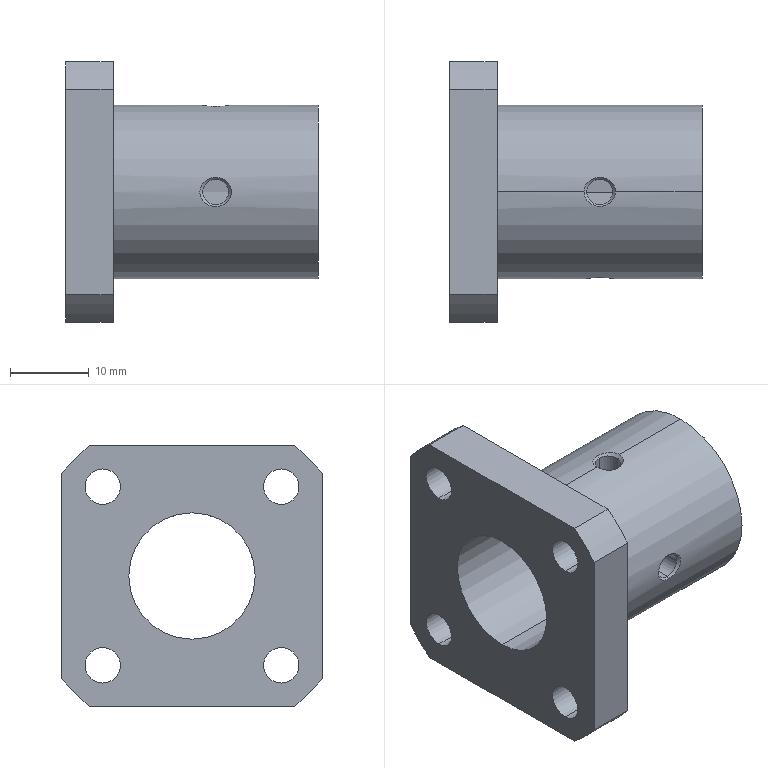Part | STEP file | STHSB16_STHSB16 | 1 solid | 41 faces | box 32 x 33 x 33 mm | volume 9412 mm3 | cylinder 26 | cone 8 | plane 7 | commonest cylinder face diameters 4.5 x8 4 x6 3.242 x4 42 x4 16 x2 22 x2
STEP:
#1=CARTESIAN_POINT('',(19.,-1.621,10.621));
#2=VERTEX_POINT('',#1);
#3=CARTESIAN_POINT('',(19.,1.621,10.621));
#4=VERTEX_POINT('',#3);
#5=CARTESIAN_POINT('',(19.,0.,10.621));
#6=DIRECTION('',(0.,0.,-1.));
#7=DIRECTION('',(0.,1.,0.));
#8=AXIS2_PLACEMENT_3D('',#5,#6,#7);
#9=CIRCLE('',#8,1.621);
#10=EDGE_CURVE('',#2,#4,#9,.T.);
#11=ORIENTED_EDGE('',*,*,#10,.F.);
#12=CARTESIAN_POINT('',(19.,-1.621,8.379));
#13=VERTEX_POINT('',#12);
#14=CARTESIAN_POINT('',(19.,-1.621,11.8));
#15=DIRECTION('',(0.,0.,-1.));
#16=VECTOR('',#15,1000.);
#17=LINE('',#14,#16);
#18=EDGE_CURVE('',#2,#13,#17,.T.);
#19=ORIENTED_EDGE('',*,*,#18,.T.);
#20=CARTESIAN_POINT('',(19.,1.621,8.379));
#21=VERTEX_POINT('',#20);
#22=CARTESIAN_POINT('',(19.,0.,8.379));
#23=DIRECTION('',(0.,0.,-1.));
#24=DIRECTION('',(0.,1.,0.));
#25=AXIS2_PLACEMENT_3D('',#22,#23,#24);
#26=CIRCLE('',#25,1.621);
#27=EDGE_CURVE('',#13,#21,#26,.T.);
#28=ORIENTED_EDGE('',*,*,#27,.T.);
#29=CARTESIAN_POINT('',(19.,1.621,11.8));
#30=DIRECTION('',(0.,0.,-1.));
#31=VECTOR('',#30,1000.);
#32=LINE('',#29,#31);
#33=EDGE_CURVE('',#4,#21,#32,.T.);
#34=ORIENTED_EDGE('',*,*,#33,.F.);
#35=EDGE_LOOP('',(#11,#19,#28,#34));
#36=FACE_OUTER_BOUND('',#35,.T.);
#37=CARTESIAN_POINT('',(19.,0.,11.8));
#38=DIRECTION('',(0.,0.,-1.));
#39=DIRECTION('',(0.,1.,0.));
#40=AXIS2_PLACEMENT_3D('',#37,#38,#39);
#41=CYLINDRICAL_SURFACE('',#40,1.621);
#42=ADVANCED_FACE('',(#36),#41,.F.);
#43=ORIENTED_EDGE('',*,*,#27,.F.);
#44=CARTESIAN_POINT('',(19.,-2.,8.));
#45=VERTEX_POINT('',#44);
#46=CARTESIAN_POINT('',(19.,-1.621,8.379));
#47=DIRECTION('',(0.,-0.7071,-0.7071));
#48=VECTOR('',#47,1000.);
#49=LINE('',#46,#48);
#50=EDGE_CURVE('',#13,#45,#49,.T.);
#51=ORIENTED_EDGE('',*,*,#50,.T.);
#52=CARTESIAN_POINT('',(17.,0.,8.));
#53=VERTEX_POINT('',#52);
#54=CARTESIAN_POINT('',(19.,0.,8.));
#55=DIRECTION('',(0.,0.,-1.));
#56=DIRECTION('',(0.,1.,0.));
#57=AXIS2_PLACEMENT_3D('',#54,#55,#56);
#58=CIRCLE('',#57,2.);
#59=EDGE_CURVE('',#45,#53,#58,.T.);
#60=ORIENTED_EDGE('',*,*,#59,.T.);
#61=CARTESIAN_POINT('',(19.,2.,8.));
#62=VERTEX_POINT('',#61);
#63=CARTESIAN_POINT('',(19.,0.,8.));
#64=DIRECTION('',(0.,0.,-1.));
#65=DIRECTION('',(0.,1.,0.));
#66=AXIS2_PLACEMENT_3D('',#63,#64,#65);
#67=CIRCLE('',#66,2.);
#68=EDGE_CURVE('',#53,#62,#67,.T.);
#69=ORIENTED_EDGE('',*,*,#68,.T.);
#70=CARTESIAN_POINT('',(19.,1.621,8.379));
#71=DIRECTION('',(0.,0.7071,-0.7071));
#72=VECTOR('',#71,1000.);
#73=LINE('',#70,#72);
#74=EDGE_CURVE('',#21,#62,#73,.T.);
#75=ORIENTED_EDGE('',*,*,#74,.F.);
#76=EDGE_LOOP('',(#43,#51,#60,#69,#75));
#77=FACE_OUTER_BOUND('',#76,.T.);
#78=CARTESIAN_POINT('',(19.,0.,8.379));
#79=DIRECTION('',(0.,0.,-1.));
#80=DIRECTION('',(0.,1.,0.));
#81=AXIS2_PLACEMENT_3D('',#78,#79,#80);
#82=CONICAL_SURFACE('',#81,1.621,0.7854);
#83=ADVANCED_FACE('',(#77),#82,.F.);
#84=ORIENTED_EDGE('',*,*,#10,.T.);
#85=CARTESIAN_POINT('',(19.,1.844,10.844));
#86=VERTEX_POINT('',#85);
#87=CARTESIAN_POINT('',(19.,2.,11.));
#88=DIRECTION('',(0.,0.7071,0.7071));
#89=VECTOR('',#88,1000.);
#90=LINE('',#87,#89);
#91=EDGE_CURVE('',#4,#86,#90,.T.);
#92=ORIENTED_EDGE('',*,*,#91,.T.);
#93=CARTESIAN_POINT('',(17.,0.,11.));
#94=VERTEX_POINT('',#93);
#95=CARTESIAN_POINT('',(19.,1.844,10.844));
#96=CARTESIAN_POINT('',(18.874,1.844,10.844));
#97=CARTESIAN_POINT('',(18.747,1.833,10.846));
#98=CARTESIAN_POINT('',(18.499,1.789,10.854));
#99=CARTESIAN_POINT('',(18.378,1.756,10.859));
#100=CARTESIAN_POINT('',(18.142,1.669,10.873));
#101=CARTESIAN_POINT('',(18.027,1.615,10.881));
#102=CARTESIAN_POINT('',(17.811,1.486,10.899));
#103=CARTESIAN_POINT('',(17.71,1.413,10.909));
#104=CARTESIAN_POINT('',(17.522,1.247,10.929));
#105=CARTESIAN_POINT('',(17.435,1.153,10.94));
#106=CARTESIAN_POINT('',(17.284,0.9535,10.959));
#107=CARTESIAN_POINT('',(17.219,0.8468,10.968));
#108=CARTESIAN_POINT('',(17.058,0.5039,10.991));
#109=CARTESIAN_POINT('',(17.,0.2536,11.));
#110=CARTESIAN_POINT('',(17.,0.,11.));
#111=B_SPLINE_CURVE_WITH_KNOTS('',3,(#95,#96,#97,#98,#99,#100,#101,#102,#103,#104,#105,#106,#107,#108,#109,#110),.UNSPECIFIED.,.F.,.F.,(4,2,2,2,2,2,2,4),(0.007522,0.0079,0.008277,0.008655,0.009033,0.009411,0.009788,0.01054),.UNSPECIFIED.);
#112=EDGE_CURVE('',#86,#94,#111,.T.);
#113=ORIENTED_EDGE('',*,*,#112,.T.);
#114=CARTESIAN_POINT('',(19.,-1.844,10.844));
#115=VERTEX_POINT('',#114);
#116=CARTESIAN_POINT('',(17.,0.,11.));
#117=CARTESIAN_POINT('',(17.,-0.1265,11.));
#118=CARTESIAN_POINT('',(17.014,-0.2511,10.998));
#119=CARTESIAN_POINT('',(17.069,-0.4966,10.989));
#120=CARTESIAN_POINT('',(17.111,-0.6176,10.983));
#121=CARTESIAN_POINT('',(17.271,-0.958,10.961));
#122=CARTESIAN_POINT('',(17.427,-1.163,10.94));
#123=CARTESIAN_POINT('',(17.711,-1.414,10.909));
#124=CARTESIAN_POINT('',(17.813,-1.488,10.899));
#125=CARTESIAN_POINT('',(18.029,-1.616,10.881));
#126=CARTESIAN_POINT('',(18.144,-1.67,10.873));
#127=CARTESIAN_POINT('',(18.379,-1.757,10.859));
#128=CARTESIAN_POINT('',(18.5,-1.789,10.854));
#129=CARTESIAN_POINT('',(18.748,-1.833,10.846));
#130=CARTESIAN_POINT('',(18.875,-1.844,10.844));
#131=CARTESIAN_POINT('',(19.,-1.844,10.844));
#132=B_SPLINE_CURVE_WITH_KNOTS('',3,(#116,#117,#118,#119,#120,#121,#122,#123,#124,#125,#126,#127,#128,#129,#130,#131),.UNSPECIFIED.,.F.,.F.,(4,2,2,2,2,2,2,4),(0.01054,0.01092,0.0113,0.01205,0.01243,0.01281,0.01318,0.01356),.UNSPECIFIED.);
#133=EDGE_CURVE('',#94,#115,#132,.T.);
#134=ORIENTED_EDGE('',*,*,#133,.T.);
#135=CARTESIAN_POINT('',(19.,-2.,11.));
#136=DIRECTION('',(0.,-0.7071,0.7071));
#137=VECTOR('',#136,1000.);
#138=LINE('',#135,#137);
#139=EDGE_CURVE('',#2,#115,#138,.T.);
#140=ORIENTED_EDGE('',*,*,#139,.F.);
#141=EDGE_LOOP('',(#84,#92,#113,#134,#140));
#142=FACE_OUTER_BOUND('',#141,.T.);
#143=CARTESIAN_POINT('',(19.,0.,11.));
#144=DIRECTION('',(0.,0.,1.));
#145=DIRECTION('',(0.,-1.,0.));
#146=AXIS2_PLACEMENT_3D('',#143,#144,#145);
#147=CONICAL_SURFACE('',#146,2.,0.7854);
#148=ADVANCED_FACE('',(#142),#147,.F.);
#149=CARTESIAN_POINT('',(21.,0.,8.));
#150=VERTEX_POINT('',#149);
#151=CARTESIAN_POINT('',(19.,0.,8.));
#152=DIRECTION('',(0.,0.,-1.));
#153=DIRECTION('',(0.,1.,0.));
#154=AXIS2_PLACEMENT_3D('',#151,#152,#153);
#155=CIRCLE('',#154,2.);
#156=EDGE_CURVE('',#62,#150,#155,.T.);
#157=ORIENTED_EDGE('',*,*,#156,.F.);
#158=CARTESIAN_POINT('',(19.,2.,7.746));
#159=VERTEX_POINT('',#158);
#160=CARTESIAN_POINT('',(19.,2.,11.8));
#161=DIRECTION('',(0.,0.,-1.));
#162=VECTOR('',#161,1000.);
#163=LINE('',#160,#162);
#164=EDGE_CURVE('',#62,#159,#163,.T.);
#165=ORIENTED_EDGE('',*,*,#164,.T.);
#166=CARTESIAN_POINT('',(19.,2.,7.746));
#167=CARTESIAN_POINT('',(19.132,2.,7.746));
#168=CARTESIAN_POINT('',(19.262,1.987,7.749));
#169=CARTESIAN_POINT('',(19.519,1.936,7.762));
#170=CARTESIAN_POINT('',(19.646,1.897,7.772));
#171=CARTESIAN_POINT('',(20.008,1.747,7.808));
#172=CARTESIAN_POINT('',(20.23,1.598,7.841));
#173=CARTESIAN_POINT('',(20.597,1.231,7.907));
#174=CARTESIAN_POINT('',(20.746,1.009,7.94));
#175=CARTESIAN_POINT('',(20.896,0.6485,7.975));
#176=CARTESIAN_POINT('',(20.935,0.5211,7.984));
#177=CARTESIAN_POINT('',(20.987,0.2634,7.997));
#178=CARTESIAN_POINT('',(21.,0.1326,8.));
#179=CARTESIAN_POINT('',(21.,0.,8.));
#180=B_SPLINE_CURVE_WITH_KNOTS('',3,(#166,#167,#168,#169,#170,#171,#172,#173,#174,#175,#176,#177,#178,#179),.UNSPECIFIED.,.F.,.F.,(4,2,2,2,2,2,4),(0.009417,0.009809,0.0102,0.01099,0.01177,0.01216,0.01255),.UNSPECIFIED.);
#181=EDGE_CURVE('',#159,#150,#180,.T.);
#182=ORIENTED_EDGE('',*,*,#181,.T.);
#183=EDGE_LOOP('',(#157,#165,#182));
#184=FACE_OUTER_BOUND('',#183,.T.);
#185=CARTESIAN_POINT('',(19.,0.,11.8));
#186=DIRECTION('',(0.,0.,-1.));
#187=DIRECTION('',(0.,1.,0.));
#188=AXIS2_PLACEMENT_3D('',#185,#186,#187);
#189=CYLINDRICAL_SURFACE('',#188,2.);
#190=ADVANCED_FACE('',(#184),#189,.F.);
#191=CARTESIAN_POINT('',(19.,-10.621,-1.621));
#192=VERTEX_POINT('',#191);
#193=CARTESIAN_POINT('',(19.,-10.621,1.621));
#194=VERTEX_POINT('',#193);
#195=CARTESIAN_POINT('',(19.,-10.621,0.));
#196=DIRECTION('',(0.,1.,0.));
#197=DIRECTION('',(0.,0.,1.));
#198=AXIS2_PLACEMENT_3D('',#195,#196,#197);
#199=CIRCLE('',#198,1.621);
#200=EDGE_CURVE('',#192,#194,#199,.T.);
#201=ORIENTED_EDGE('',*,*,#200,.F.);
#202=CARTESIAN_POINT('',(19.,-8.379,-1.621));
#203=VERTEX_POINT('',#202);
#204=CARTESIAN_POINT('',(19.,-11.8,-1.621));
#205=DIRECTION('',(0.,1.,0.));
#206=VECTOR('',#205,1000.);
#207=LINE('',#204,#206);
#208=EDGE_CURVE('',#192,#203,#207,.T.);
#209=ORIENTED_EDGE('',*,*,#208,.T.);
#210=CARTESIAN_POINT('',(19.,-8.379,1.621));
#211=VERTEX_POINT('',#210);
#212=CARTESIAN_POINT('',(19.,-8.379,0.));
#213=DIRECTION('',(0.,1.,0.));
#214=DIRECTION('',(0.,0.,1.));
#215=AXIS2_PLACEMENT_3D('',#212,#213,#214);
#216=CIRCLE('',#215,1.621);
#217=EDGE_CURVE('',#203,#211,#216,.T.);
#218=ORIENTED_EDGE('',*,*,#217,.T.);
#219=CARTESIAN_POINT('',(19.,-11.8,1.621));
#220=DIRECTION('',(0.,1.,0.));
#221=VECTOR('',#220,1000.);
#222=LINE('',#219,#221);
#223=EDGE_CURVE('',#194,#211,#222,.T.);
#224=ORIENTED_EDGE('',*,*,#223,.F.);
#225=EDGE_LOOP('',(#201,#209,#218,#224));
#226=FACE_OUTER_BOUND('',#225,.T.);
#227=CARTESIAN_POINT('',(19.,-11.8,0.));
#228=DIRECTION('',(0.,1.,0.));
#229=DIRECTION('',(0.,0.,1.));
#230=AXIS2_PLACEMENT_3D('',#227,#228,#229);
#231=CYLINDRICAL_SURFACE('',#230,1.621);
#232=ADVANCED_FACE('',(#226),#231,.F.);
#233=ORIENTED_EDGE('',*,*,#217,.F.);
#234=CARTESIAN_POINT('',(19.,-8.,-2.));
#235=VERTEX_POINT('',#234);
#236=CARTESIAN_POINT('',(19.,-8.379,-1.621));
#237=DIRECTION('',(0.,0.7071,-0.7071));
#238=VECTOR('',#237,1000.);
#239=LINE('',#236,#238);
#240=EDGE_CURVE('',#203,#235,#239,.T.);
#241=ORIENTED_EDGE('',*,*,#240,.T.);
#242=CARTESIAN_POINT('',(17.,-8.,0.));
#243=VERTEX_POINT('',#242);
#244=CARTESIAN_POINT('',(19.,-8.,0.));
#245=DIRECTION('',(0.,1.,0.));
#246=DIRECTION('',(0.,0.,1.));
#247=AXIS2_PLACEMENT_3D('',#244,#245,#246);
#248=CIRCLE('',#247,2.);
#249=EDGE_CURVE('',#235,#243,#248,.T.);
#250=ORIENTED_EDGE('',*,*,#249,.T.);
#251=CARTESIAN_POINT('',(19.,-8.,2.));
#252=VERTEX_POINT('',#251);
#253=CARTESIAN_POINT('',(19.,-8.,0.));
#254=DIRECTION('',(0.,1.,0.));
#255=DIRECTION('',(0.,0.,1.));
#256=AXIS2_PLACEMENT_3D('',#253,#254,#255);
#257=CIRCLE('',#256,2.);
#258=EDGE_CURVE('',#243,#252,#257,.T.);
#259=ORIENTED_EDGE('',*,*,#258,.T.);
#260=CARTESIAN_POINT('',(19.,-8.379,1.621));
#261=DIRECTION('',(0.,0.7071,0.7071));
#262=VECTOR('',#261,1000.);
#263=LINE('',#260,#262);
#264=EDGE_CURVE('',#211,#252,#263,.T.);
#265=ORIENTED_EDGE('',*,*,#264,.F.);
#266=EDGE_LOOP('',(#233,#241,#250,#259,#265));
#267=FACE_OUTER_BOUND('',#266,.T.);
#268=CARTESIAN_POINT('',(19.,-8.379,0.));
#269=DIRECTION('',(0.,1.,0.));
#270=DIRECTION('',(0.,0.,1.));
#271=AXIS2_PLACEMENT_3D('',#268,#269,#270);
#272=CONICAL_SURFACE('',#271,1.621,0.7854);
#273=ADVANCED_FACE('',(#267),#272,.F.);
#274=ORIENTED_EDGE('',*,*,#200,.T.);
#275=CARTESIAN_POINT('',(19.,-10.844,1.844));
#276=VERTEX_POINT('',#275);
#277=CARTESIAN_POINT('',(19.,-11.,2.));
#278=DIRECTION('',(0.,-0.7071,0.7071));
#279=VECTOR('',#278,1000.);
#280=LINE('',#277,#279);
#281=EDGE_CURVE('',#194,#276,#280,.T.);
#282=ORIENTED_EDGE('',*,*,#281,.T.);
#283=CARTESIAN_POINT('',(19.,-10.844,-1.844));
#284=VERTEX_POINT('',#283);
#285=CARTESIAN_POINT('',(19.,-10.844,1.844));
#286=CARTESIAN_POINT('',(18.874,-10.844,1.844));
#287=CARTESIAN_POINT('',(18.747,-10.846,1.833));
#288=CARTESIAN_POINT('',(18.499,-10.854,1.789));
#289=CARTESIAN_POINT('',(18.379,-10.859,1.756));
#290=CARTESIAN_POINT('',(18.143,-10.873,1.67));
#291=CARTESIAN_POINT('',(18.028,-10.881,1.615));
#292=CARTESIAN_POINT('',(17.812,-10.899,1.487));
#293=CARTESIAN_POINT('',(17.711,-10.909,1.414));
#294=CARTESIAN_POINT('',(17.523,-10.929,1.248));
#295=CARTESIAN_POINT('',(17.436,-10.94,1.154));
#296=CARTESIAN_POINT('',(17.285,-10.959,0.9553));
#297=CARTESIAN_POINT('',(17.22,-10.968,0.8487));
#298=CARTESIAN_POINT('',(17.058,-10.991,0.5066));
#299=CARTESIAN_POINT('',(17.,-11.,0.2567));
#300=CARTESIAN_POINT('',(17.,-11.,-0.1234));
#301=CARTESIAN_POINT('',(17.014,-10.998,-0.2482));
#302=CARTESIAN_POINT('',(17.069,-10.99,-0.494));
#303=CARTESIAN_POINT('',(17.11,-10.983,-0.6152));
#304=CARTESIAN_POINT('',(17.27,-10.961,-0.9562));
#305=CARTESIAN_POINT('',(17.426,-10.94,-1.161));
#306=CARTESIAN_POINT('',(17.71,-10.909,-1.413));
#307=CARTESIAN_POINT('',(17.812,-10.899,-1.487));
#308=CARTESIAN_POINT('',(18.028,-10.881,-1.615));
#309=CARTESIAN_POINT('',(18.143,-10.873,-1.67));
#310=CARTESIAN_POINT('',(18.379,-10.859,-1.757));
#311=CARTESIAN_POINT('',(18.5,-10.854,-1.789));
#312=CARTESIAN_POINT('',(18.747,-10.846,-1.833));
#313=CARTESIAN_POINT('',(18.875,-10.844,-1.844));
#314=CARTESIAN_POINT('',(19.,-10.844,-1.844));
#315=B_SPLINE_CURVE_WITH_KNOTS('',3,(#285,#286,#287,#288,#289,#290,#291,#292,#293,#294,#295,#296,#297,#298,#299,#300,#301,#302,#303,#304,#305,#306,#307,#308,#309,#310,#311,#312,#313,#314),.UNSPECIFIED.,.F.,.F.,(4,2,2,2,2,2,2,2,2,2,2,2,2,2,4),(0.007522,0.007899,0.008277,0.008654,0.009031,0.009409,0.009786,0.01054,0.01092,0.0113,0.01205,0.01243,0.0128,0.01318,0.01356),.UNSPECIFIED.);
#316=EDGE_CURVE('',#276,#284,#315,.T.);
#317=ORIENTED_EDGE('',*,*,#316,.T.);
#318=CARTESIAN_POINT('',(19.,-11.,-2.));
#319=DIRECTION('',(0.,-0.7071,-0.7071));
#320=VECTOR('',#319,1000.);
#321=LINE('',#318,#320);
#322=EDGE_CURVE('',#192,#284,#321,.T.);
#323=ORIENTED_EDGE('',*,*,#322,.F.);
#324=EDGE_LOOP('',(#274,#282,#317,#323));
#325=FACE_OUTER_BOUND('',#324,.T.);
#326=CARTESIAN_POINT('',(19.,-11.,0.));
#327=DIRECTION('',(0.,-1.,0.));
#328=DIRECTION('',(0.,0.,-1.));
#329=AXIS2_PLACEMENT_3D('',#326,#327,#328);
#330=CONICAL_SURFACE('',#329,2.,0.7854);
#331=ADVANCED_FACE('',(#325),#330,.F.);
#332=CARTESIAN_POINT('',(21.,-8.,0.));
#333=VERTEX_POINT('',#332);
#334=CARTESIAN_POINT('',(19.,-8.,0.));
#335=DIRECTION('',(0.,1.,0.));
#336=DIRECTION('',(0.,0.,1.));
#337=AXIS2_PLACEMENT_3D('',#334,#335,#336);
#338=CIRCLE('',#337,2.);
#339=EDGE_CURVE('',#252,#333,#338,.T.);
#340=ORIENTED_EDGE('',*,*,#339,.F.);
#341=CARTESIAN_POINT('',(19.,-7.746,2.));
#342=VERTEX_POINT('',#341);
#343=CARTESIAN_POINT('',(19.,-11.8,2.));
#344=DIRECTION('',(0.,1.,0.));
#345=VECTOR('',#344,1000.);
#346=LINE('',#343,#345);
#347=EDGE_CURVE('',#252,#342,#346,.T.);
#348=ORIENTED_EDGE('',*,*,#347,.T.);
#349=CARTESIAN_POINT('',(19.,-7.746,2.));
#350=CARTESIAN_POINT('',(19.131,-7.746,2.));
#351=CARTESIAN_POINT('',(19.264,-7.749,1.987));
#352=CARTESIAN_POINT('',(19.521,-7.762,1.935));
#353=CARTESIAN_POINT('',(19.646,-7.772,1.897));
#354=CARTESIAN_POINT('',(20.01,-7.808,1.746));
#355=CARTESIAN_POINT('',(20.23,-7.841,1.599));
#356=CARTESIAN_POINT('',(20.507,-7.891,1.321));
#357=CARTESIAN_POINT('',(20.59,-7.907,1.221));
#358=CARTESIAN_POINT('',(20.734,-7.937,1.004));
#359=CARTESIAN_POINT('',(20.797,-7.952,0.8872));
#360=CARTESIAN_POINT('',(20.897,-7.975,0.6458));
#361=CARTESIAN_POINT('',(20.935,-7.984,0.5211));
#362=CARTESIAN_POINT('',(20.987,-7.997,0.2636));
#363=CARTESIAN_POINT('',(21.,-8.,0.1308));
#364=CARTESIAN_POINT('',(21.,-8.,0.));
#365=B_SPLINE_CURVE_WITH_KNOTS('',3,(#349,#350,#351,#352,#353,#354,#355,#356,#357,#358,#359,#360,#361,#362,#363,#364),.UNSPECIFIED.,.F.,.F.,(4,2,2,2,2,2,2,4),(0.00314,0.003532,0.003924,0.004709,0.005101,0.005493,0.005886,0.006278),.UNSPECIFIED.);
#366=EDGE_CURVE('',#342,#333,#365,.T.);
#367=ORIENTED_EDGE('',*,*,#366,.T.);
#368=EDGE_LOOP('',(#340,#348,#367));
#369=FACE_OUTER_BOUND('',#368,.T.);
#370=CARTESIAN_POINT('',(19.,-11.8,0.));
#371=DIRECTION('',(0.,1.,0.));
#372=DIRECTION('',(0.,0.,1.));
#373=AXIS2_PLACEMENT_3D('',#370,#371,#372);
#374=CYLINDRICAL_SURFACE('',#373,2.);
#375=ADVANCED_FACE('',(#369),#374,.F.);
#376=CARTESIAN_POINT('',(6.,-11.314,13.564));
#377=VERTEX_POINT('',#376);
#378=CARTESIAN_POINT('',(6.,-11.314,9.064));
#379=VERTEX_POINT('',#378);
#380=CARTESIAN_POINT('',(6.,-11.314,11.314));
#381=DIRECTION('',(1.,0.,0.));
#382=DIRECTION('',(0.,0.,-1.));
#383=AXIS2_PLACEMENT_3D('',#380,#381,#382);
#384=CIRCLE('',#383,2.25);
#385=EDGE_CURVE('',#377,#379,#384,.T.);
#386=ORIENTED_EDGE('',*,*,#385,.T.);
#387=CARTESIAN_POINT('',(0.,-11.314,9.064));
#388=VERTEX_POINT('',#387);
#389=CARTESIAN_POINT('',(6.,-11.314,9.064));
#390=DIRECTION('',(-1.,0.,0.));
#391=VECTOR('',#390,1000.);
#392=LINE('',#389,#391);
#393=EDGE_CURVE('',#379,#388,#392,.T.);
#394=ORIENTED_EDGE('',*,*,#393,.T.);
#395=CARTESIAN_POINT('',(0.,-11.314,13.564));
#396=VERTEX_POINT('',#395);
#397=CARTESIAN_POINT('',(0.,-11.314,11.314));
#398=DIRECTION('',(1.,0.,0.));
#399=DIRECTION('',(0.,0.,-1.));
#400=AXIS2_PLACEMENT_3D('',#397,#398,#399);
#401=CIRCLE('',#400,2.25);
#402=EDGE_CURVE('',#396,#388,#401,.T.);
#403=ORIENTED_EDGE('',*,*,#402,.F.);
#404=CARTESIAN_POINT('',(6.,-11.314,13.564));
#405=DIRECTION('',(-1.,0.,0.));
#406=VECTOR('',#405,1000.);
#407=LINE('',#404,#406);
#408=EDGE_CURVE('',#377,#396,#407,.T.);
#409=ORIENTED_EDGE('',*,*,#408,.F.);
#410=EDGE_LOOP('',(#386,#394,#403,#409));
#411=FACE_OUTER_BOUND('',#410,.T.);
#412=CARTESIAN_POINT('',(6.,-11.314,11.314));
#413=DIRECTION('',(-1.,0.,0.));
#414=DIRECTION('',(0.,0.,1.));
#415=AXIS2_PLACEMENT_3D('',#412,#413,#414);
#416=CYLINDRICAL_SURFACE('',#415,2.25);
#417=ADVANCED_FACE('',(#411),#416,.F.);
#418=CARTESIAN_POINT('',(6.,11.314,13.564));
#419=VERTEX_POINT('',#418);
#420=CARTESIAN_POINT('',(6.,11.314,9.064));
#421=VERTEX_POINT('',#420);
#422=CARTESIAN_POINT('',(6.,11.314,11.314));
#423=DIRECTION('',(1.,0.,0.));
#424=DIRECTION('',(0.,0.,-1.));
#425=AXIS2_PLACEMENT_3D('',#422,#423,#424);
#426=CIRCLE('',#425,2.25);
#427=EDGE_CURVE('',#419,#421,#426,.T.);
#428=ORIENTED_EDGE('',*,*,#427,.T.);
#429=CARTESIAN_POINT('',(0.,11.314,9.064));
#430=VERTEX_POINT('',#429);
#431=CARTESIAN_POINT('',(6.,11.314,9.064));
#432=DIRECTION('',(-1.,0.,0.));
#433=VECTOR('',#432,1000.);
#434=LINE('',#431,#433);
#435=EDGE_CURVE('',#421,#430,#434,.T.);
#436=ORIENTED_EDGE('',*,*,#435,.T.);
#437=CARTESIAN_POINT('',(0.,11.314,13.564));
#438=VERTEX_POINT('',#437);
#439=CARTESIAN_POINT('',(0.,11.314,11.314));
#440=DIRECTION('',(1.,0.,0.));
#441=DIRECTION('',(0.,0.,-1.));
#442=AXIS2_PLACEMENT_3D('',#439,#440,#441);
#443=CIRCLE('',#442,2.25);
#444=EDGE_CURVE('',#438,#430,#443,.T.);
#445=ORIENTED_EDGE('',*,*,#444,.F.);
#446=CARTESIAN_POINT('',(6.,11.314,13.564));
#447=DIRECTION('',(-1.,0.,0.));
#448=VECTOR('',#447,1000.);
#449=LINE('',#446,#448);
#450=EDGE_CURVE('',#419,#438,#449,.T.);
#451=ORIENTED_EDGE('',*,*,#450,.F.);
#452=EDGE_LOOP('',(#428,#436,#445,#451));
#453=FACE_OUTER_BOUND('',#452,.T.);
#454=CARTESIAN_POINT('',(6.,11.314,11.314));
#455=DIRECTION('',(-1.,0.,0.));
#456=DIRECTION('',(0.,0.,1.));
#457=AXIS2_PLACEMENT_3D('',#454,#455,#456);
#458=CYLINDRICAL_SURFACE('',#457,2.25);
#459=ADVANCED_FACE('',(#453),#458,.F.);
#460=CARTESIAN_POINT('',(6.,-11.314,-9.064));
#461=VERTEX_POINT('',#460);
#462=CARTESIAN_POINT('',(6.,-11.314,-13.564));
#463=VERTEX_POINT('',#462);
#464=CARTESIAN_POINT('',(6.,-11.314,-11.314));
#465=DIRECTION('',(1.,0.,0.));
#466=DIRECTION('',(0.,0.,-1.));
#467=AXIS2_PLACEMENT_3D('',#464,#465,#466);
#468=CIRCLE('',#467,2.25);
#469=EDGE_CURVE('',#461,#463,#468,.T.);
#470=ORIENTED_EDGE('',*,*,#469,.T.);
#471=CARTESIAN_POINT('',(0.,-11.314,-13.564));
#472=VERTEX_POINT('',#471);
#473=CARTESIAN_POINT('',(6.,-11.314,-13.564));
#474=DIRECTION('',(-1.,0.,0.));
#475=VECTOR('',#474,1000.);
#476=LINE('',#473,#475);
#477=EDGE_CURVE('',#463,#472,#476,.T.);
#478=ORIENTED_EDGE('',*,*,#477,.T.);
#479=CARTESIAN_POINT('',(0.,-11.314,-9.064));
#480=VERTEX_POINT('',#479);
#481=CARTESIAN_POINT('',(0.,-11.314,-11.314));
#482=DIRECTION('',(1.,0.,0.));
#483=DIRECTION('',(0.,0.,-1.));
#484=AXIS2_PLACEMENT_3D('',#481,#482,#483);
#485=CIRCLE('',#484,2.25);
#486=EDGE_CURVE('',#480,#472,#485,.T.);
#487=ORIENTED_EDGE('',*,*,#486,.F.);
#488=CARTESIAN_POINT('',(6.,-11.314,-9.064));
#489=DIRECTION('',(-1.,0.,0.));
#490=VECTOR('',#489,1000.);
#491=LINE('',#488,#490);
#492=EDGE_CURVE('',#461,#480,#491,.T.);
#493=ORIENTED_EDGE('',*,*,#492,.F.);
#494=EDGE_LOOP('',(#470,#478,#487,#493));
#495=FACE_OUTER_BOUND('',#494,.T.);
#496=CARTESIAN_POINT('',(6.,-11.314,-11.314));
#497=DIRECTION('',(-1.,0.,0.));
#498=DIRECTION('',(0.,0.,1.));
#499=AXIS2_PLACEMENT_3D('',#496,#497,#498);
#500=CYLINDRICAL_SURFACE('',#499,2.25);
#501=ADVANCED_FACE('',(#495),#500,.F.);
#502=CARTESIAN_POINT('',(6.,11.314,-9.064));
#503=VERTEX_POINT('',#502);
#504=CARTESIAN_POINT('',(6.,11.314,-13.564));
#505=VERTEX_POINT('',#504);
#506=CARTESIAN_POINT('',(6.,11.314,-11.314));
#507=DIRECTION('',(1.,0.,0.));
#508=DIRECTION('',(0.,0.,-1.));
#509=AXIS2_PLACEMENT_3D('',#506,#507,#508);
#510=CIRCLE('',#509,2.25);
#511=EDGE_CURVE('',#503,#505,#510,.T.);
#512=ORIENTED_EDGE('',*,*,#511,.T.);
#513=CARTESIAN_POINT('',(0.,11.314,-13.564));
#514=VERTEX_POINT('',#513);
#515=CARTESIAN_POINT('',(6.,11.314,-13.564));
#516=DIRECTION('',(-1.,0.,0.));
#517=VECTOR('',#516,1000.);
#518=LINE('',#515,#517);
#519=EDGE_CURVE('',#505,#514,#518,.T.);
#520=ORIENTED_EDGE('',*,*,#519,.T.);
#521=CARTESIAN_POINT('',(0.,11.314,-9.064));
#522=VERTEX_POINT('',#521);
#523=CARTESIAN_POINT('',(0.,11.314,-11.314));
#524=DIRECTION('',(1.,0.,0.));
#525=DIRECTION('',(0.,0.,-1.));
#526=AXIS2_PLACEMENT_3D('',#523,#524,#525);
#527=CIRCLE('',#526,2.25);
#528=EDGE_CURVE('',#522,#514,#527,.T.);
#529=ORIENTED_EDGE('',*,*,#528,.F.);
#530=CARTESIAN_POINT('',(6.,11.314,-9.064));
#531=DIRECTION('',(-1.,0.,0.));
#532=VECTOR('',#531,1000.);
#533=LINE('',#530,#532);
#534=EDGE_CURVE('',#503,#522,#533,.T.);
#535=ORIENTED_EDGE('',*,*,#534,.F.);
#536=EDGE_LOOP('',(#512,#520,#529,#535));
#537=FACE_OUTER_BOUND('',#536,.T.);
#538=CARTESIAN_POINT('',(6.,11.314,-11.314));
#539=DIRECTION('',(-1.,0.,0.));
#540=DIRECTION('',(0.,0.,1.));
#541=AXIS2_PLACEMENT_3D('',#538,#539,#540);
#542=CYLINDRICAL_SURFACE('',#541,2.25);
#543=ADVANCED_FACE('',(#537),#542,.F.);
#544=CARTESIAN_POINT('',(32.,0.,11.));
#545=VERTEX_POINT('',#544);
#546=CARTESIAN_POINT('',(32.,0.,-11.));
#547=VERTEX_POINT('',#546);
#548=CARTESIAN_POINT('',(32.,0.,0.));
#549=DIRECTION('',(-1.,0.,0.));
#550=DIRECTION('',(0.,0.,1.));
#551=AXIS2_PLACEMENT_3D('',#548,#549,#550);
#552=CIRCLE('',#551,11.);
#553=EDGE_CURVE('',#545,#547,#552,.T.);
#554=ORIENTED_EDGE('',*,*,#553,.T.);
#555=CARTESIAN_POINT('',(6.,0.,-11.));
#556=VERTEX_POINT('',#555);
#557=CARTESIAN_POINT('',(32.,0.,-11.));
#558=DIRECTION('',(-1.,0.,0.));
#559=VECTOR('',#558,1000.);
#560=LINE('',#557,#559);
#561=EDGE_CURVE('',#547,#556,#560,.T.);
#562=ORIENTED_EDGE('',*,*,#561,.T.);
#563=CARTESIAN_POINT('',(6.,0.,11.));
#564=VERTEX_POINT('',#563);
#565=CARTESIAN_POINT('',(6.,0.,0.));
#566=DIRECTION('',(-1.,0.,0.));
#567=DIRECTION('',(0.,0.,1.));
#568=AXIS2_PLACEMENT_3D('',#565,#566,#567);
#569=CIRCLE('',#568,11.);
#570=EDGE_CURVE('',#564,#556,#569,.T.);
#571=ORIENTED_EDGE('',*,*,#570,.F.);
#572=CARTESIAN_POINT('',(32.,0.,11.));
#573=DIRECTION('',(-1.,0.,0.));
#574=VECTOR('',#573,1000.);
#575=LINE('',#572,#574);
#576=EDGE_CURVE('',#94,#564,#575,.T.);
#577=ORIENTED_EDGE('',*,*,#576,.F.);
#578=ORIENTED_EDGE('',*,*,#112,.F.);
#579=CARTESIAN_POINT('',(21.,0.,11.));
#580=VERTEX_POINT('',#579);
#581=CARTESIAN_POINT('',(21.,0.,11.));
#582=CARTESIAN_POINT('',(21.,0.1258,11.));
#583=CARTESIAN_POINT('',(20.986,0.2533,10.998));
#584=CARTESIAN_POINT('',(20.93,0.498,10.989));
#585=CARTESIAN_POINT('',(20.889,0.6178,10.983));
#586=CARTESIAN_POINT('',(20.781,0.8466,10.968));
#587=CARTESIAN_POINT('',(20.716,0.9536,10.959));
#588=CARTESIAN_POINT('',(20.564,1.154,10.94));
#589=CARTESIAN_POINT('',(20.477,1.247,10.929));
#590=CARTESIAN_POINT('',(20.196,1.496,10.899));
#591=CARTESIAN_POINT('',(19.974,1.627,10.879));
#592=CARTESIAN_POINT('',(19.622,1.756,10.859));
#593=CARTESIAN_POINT('',(19.499,1.79,10.853));
#594=CARTESIAN_POINT('',(19.25,1.833,10.846));
#595=CARTESIAN_POINT('',(19.125,1.844,10.844));
#596=CARTESIAN_POINT('',(19.,1.844,10.844));
#597=B_SPLINE_CURVE_WITH_KNOTS('',3,(#581,#582,#583,#584,#585,#586,#587,#588,#589,#590,#591,#592,#593,#594,#595,#596),.UNSPECIFIED.,.F.,.F.,(4,2,2,2,2,2,2,4),(0.004504,0.004881,0.005259,0.005636,0.006013,0.006768,0.007145,0.007522),.UNSPECIFIED.);
#598=EDGE_CURVE('',#580,#86,#597,.T.);
#599=ORIENTED_EDGE('',*,*,#598,.F.);
#600=CARTESIAN_POINT('',(32.,0.,11.));
#601=DIRECTION('',(-1.,0.,0.));
#602=VECTOR('',#601,1000.);
#603=LINE('',#600,#602);
#604=EDGE_CURVE('',#545,#580,#603,.T.);
#605=ORIENTED_EDGE('',*,*,#604,.F.);
#606=EDGE_LOOP('',(#554,#562,#571,#577,#578,#599,#605));
#607=FACE_OUTER_BOUND('',#606,.T.);
#608=CARTESIAN_POINT('',(32.,0.,0.));
#609=DIRECTION('',(-1.,0.,0.));
#610=DIRECTION('',(0.,0.,1.));
#611=AXIS2_PLACEMENT_3D('',#608,#609,#610);
#612=CYLINDRICAL_SURFACE('',#611,11.);
#613=ADVANCED_FACE('',(#607),#612,.T.);
#614=CARTESIAN_POINT('',(17.,-8.,0.));
#615=CARTESIAN_POINT('',(17.,-8.,0.1327));
#616=CARTESIAN_POINT('',(17.013,-7.997,0.2632));
#617=CARTESIAN_POINT('',(17.064,-7.984,0.5196));
#618=CARTESIAN_POINT('',(17.103,-7.975,0.647));
#619=CARTESIAN_POINT('',(17.204,-7.951,0.889));
#620=CARTESIAN_POINT('',(17.265,-7.938,1.004));
#621=CARTESIAN_POINT('',(17.41,-7.907,1.221));
#622=CARTESIAN_POINT('',(17.495,-7.89,1.323));
#623=CARTESIAN_POINT('',(17.77,-7.841,1.599));
#624=CARTESIAN_POINT('',(17.993,-7.808,1.747));
#625=CARTESIAN_POINT('',(18.354,-7.772,1.897));
#626=CARTESIAN_POINT('',(18.48,-7.762,1.936));
#627=CARTESIAN_POINT('',(18.739,-7.749,1.987));
#628=CARTESIAN_POINT('',(18.869,-7.746,2.));
#629=CARTESIAN_POINT('',(19.,-7.746,2.));
#630=B_SPLINE_CURVE_WITH_KNOTS('',3,(#614,#615,#616,#617,#618,#619,#620,#621,#622,#623,#624,#625,#626,#627,#628,#629),.UNSPECIFIED.,.F.,.F.,(4,2,2,2,2,2,2,4),(0.,0.0003925,0.0007849,0.001177,0.00157,0.002355,0.002747,0.00314),.UNSPECIFIED.);
#631=EDGE_CURVE('',#243,#342,#630,.T.);
#632=ORIENTED_EDGE('',*,*,#631,.F.);
#633=CARTESIAN_POINT('',(21.,-8.,0.));
#634=CARTESIAN_POINT('',(21.,-8.,-0.2616));
#635=CARTESIAN_POINT('',(20.947,-7.986,-0.5257));
#636=CARTESIAN_POINT('',(20.797,-7.952,-0.8871));
#637=CARTESIAN_POINT('',(20.735,-7.937,-1.004));
#638=CARTESIAN_POINT('',(20.589,-7.907,-1.221));
#639=CARTESIAN_POINT('',(20.507,-7.891,-1.321));
#640=CARTESIAN_POINT('',(20.323,-7.858,-1.506));
#641=CARTESIAN_POINT('',(20.22,-7.841,-1.59));
#642=CARTESIAN_POINT('',(20.004,-7.81,-1.734));
#643=CARTESIAN_POINT('',(19.89,-7.796,-1.796));
#644=CARTESIAN_POINT('',(19.525,-7.76,-1.948));
#645=CARTESIAN_POINT('',(19.264,-7.746,-2.));
#646=CARTESIAN_POINT('',(18.869,-7.746,-2.));
#647=CARTESIAN_POINT('',(18.739,-7.749,-1.987));
#648=CARTESIAN_POINT('',(18.482,-7.762,-1.936));
#649=CARTESIAN_POINT('',(18.354,-7.772,-1.897));
#650=CARTESIAN_POINT('',(17.992,-7.808,-1.747));
#651=CARTESIAN_POINT('',(17.77,-7.841,-1.598));
#652=CARTESIAN_POINT('',(17.403,-7.907,-1.232));
#653=CARTESIAN_POINT('',(17.254,-7.94,-1.01));
#654=CARTESIAN_POINT('',(17.104,-7.975,-0.6486));
#655=CARTESIAN_POINT('',(17.065,-7.984,-0.5212));
#656=CARTESIAN_POINT('',(17.013,-7.997,-0.2634));
#657=CARTESIAN_POINT('',(17.,-8.,-0.1327));
#658=CARTESIAN_POINT('',(17.,-8.,0.));
#659=B_SPLINE_CURVE_WITH_KNOTS('',3,(#633,#634,#635,#636,#637,#638,#639,#640,#641,#642,#643,#644,#645,#646,#647,#648,#649,#650,#651,#652,#653,#654,#655,#656,#657,#658),.UNSPECIFIED.,.F.,.F.,(4,2,2,2,2,2,2,2,2,2,2,2,4),(0.006278,0.007062,0.007455,0.007847,0.008239,0.008631,0.009416,0.009808,0.0102,0.01099,0.01177,0.01216,0.01255),.UNSPECIFIED.);
#660=EDGE_CURVE('',#333,#243,#659,.T.);
#661=ORIENTED_EDGE('',*,*,#660,.F.);
#662=ORIENTED_EDGE('',*,*,#366,.F.);
#663=EDGE_LOOP('',(#632,#661,#662));
#664=FACE_BOUND('',#663,.T.);
#665=CARTESIAN_POINT('',(32.,0.,-8.));
#666=VERTEX_POINT('',#665);
#667=CARTESIAN_POINT('',(32.,0.,8.));
#668=VERTEX_POINT('',#667);
#669=CARTESIAN_POINT('',(32.,0.,0.));
#670=DIRECTION('',(-1.,0.,0.));
#671=DIRECTION('',(0.,0.,1.));
#672=AXIS2_PLACEMENT_3D('',#669,#670,#671);
#673=CIRCLE('',#672,8.);
#674=EDGE_CURVE('',#666,#668,#673,.T.);
#675=ORIENTED_EDGE('',*,*,#674,.F.);
#676=CARTESIAN_POINT('',(0.,0.,-8.));
#677=VERTEX_POINT('',#676);
#678=CARTESIAN_POINT('',(32.,0.,-8.));
#679=DIRECTION('',(-1.,0.,0.));
#680=VECTOR('',#679,1000.);
#681=LINE('',#678,#680);
#682=EDGE_CURVE('',#666,#677,#681,.T.);
#683=ORIENTED_EDGE('',*,*,#682,.T.);
#684=CARTESIAN_POINT('',(0.,0.,8.));
#685=VERTEX_POINT('',#684);
#686=CARTESIAN_POINT('',(0.,0.,0.));
#687=DIRECTION('',(-1.,0.,0.));
#688=DIRECTION('',(0.,0.,1.));
#689=AXIS2_PLACEMENT_3D('',#686,#687,#688);
#690=CIRCLE('',#689,8.);
#691=EDGE_CURVE('',#677,#685,#690,.T.);
#692=ORIENTED_EDGE('',*,*,#691,.T.);
#693=CARTESIAN_POINT('',(32.,0.,8.));
#694=DIRECTION('',(-1.,0.,0.));
#695=VECTOR('',#694,1000.);
#696=LINE('',#693,#695);
#697=EDGE_CURVE('',#53,#685,#696,.T.);
#698=ORIENTED_EDGE('',*,*,#697,.F.);
#699=CARTESIAN_POINT('',(21.,0.,8.));
#700=CARTESIAN_POINT('',(21.,-0.1327,8.));
#701=CARTESIAN_POINT('',(20.987,-0.2631,7.997));
#702=CARTESIAN_POINT('',(20.936,-0.5195,7.984));
#703=CARTESIAN_POINT('',(20.897,-0.6468,7.975));
#704=CARTESIAN_POINT('',(20.796,-0.8888,7.951));
#705=CARTESIAN_POINT('',(20.735,-1.003,7.938));
#706=CARTESIAN_POINT('',(20.59,-1.22,7.907));
#707=CARTESIAN_POINT('',(20.506,-1.323,7.89));
#708=CARTESIAN_POINT('',(20.23,-1.598,7.841));
#709=CARTESIAN_POINT('',(20.008,-1.747,7.808));
#710=CARTESIAN_POINT('',(19.647,-1.897,7.772));
#711=CARTESIAN_POINT('',(19.52,-1.936,7.762));
#712=CARTESIAN_POINT('',(19.262,-1.987,7.749));
#713=CARTESIAN_POINT('',(19.132,-2.,7.746));
#714=CARTESIAN_POINT('',(18.87,-2.,7.746));
#715=CARTESIAN_POINT('',(18.737,-1.987,7.749));
#716=CARTESIAN_POINT('',(18.48,-1.936,7.762));
#717=CARTESIAN_POINT('',(18.355,-1.898,7.772));
#718=CARTESIAN_POINT('',(17.991,-1.746,7.808));
#719=CARTESIAN_POINT('',(17.771,-1.599,7.841));
#720=CARTESIAN_POINT('',(17.493,-1.321,7.891));
#721=CARTESIAN_POINT('',(17.41,-1.221,7.907));
#722=CARTESIAN_POINT('',(17.266,-1.005,7.937));
#723=CARTESIAN_POINT('',(17.203,-0.8874,7.952));
#724=CARTESIAN_POINT('',(17.103,-0.646,7.975));
#725=CARTESIAN_POINT('',(17.065,-0.5212,7.984));
#726=CARTESIAN_POINT('',(17.013,-0.2636,7.997));
#727=CARTESIAN_POINT('',(17.,-0.1308,8.));
#728=CARTESIAN_POINT('',(17.,0.,8.));
#729=B_SPLINE_CURVE_WITH_KNOTS('',3,(#699,#700,#701,#702,#703,#704,#705,#706,#707,#708,#709,#710,#711,#712,#713,#714,#715,#716,#717,#718,#719,#720,#721,#722,#723,#724,#725,#726,#727,#728),.UNSPECIFIED.,.F.,.F.,(4,2,2,2,2,2,2,2,2,2,2,2,2,2,4),(0.,0.0003924,0.0007847,0.001177,0.001569,0.002354,0.002747,0.003139,0.003531,0.003924,0.004708,0.005101,0.005493,0.005886,0.006278),.UNSPECIFIED.);
#730=EDGE_CURVE('',#150,#53,#729,.T.);
#731=ORIENTED_EDGE('',*,*,#730,.F.);
#732=CARTESIAN_POINT('',(32.,0.,8.));
#733=DIRECTION('',(-1.,0.,0.));
#734=VECTOR('',#733,1000.);
#735=LINE('',#732,#734);
#736=EDGE_CURVE('',#668,#150,#735,.T.);
#737=ORIENTED_EDGE('',*,*,#736,.F.);
#738=EDGE_LOOP('',(#675,#683,#692,#698,#731,#737));
#739=FACE_OUTER_BOUND('',#738,.T.);
#740=CARTESIAN_POINT('',(32.,0.,0.));
#741=DIRECTION('',(-1.,0.,0.));
#742=DIRECTION('',(0.,0.,1.));
#743=AXIS2_PLACEMENT_3D('',#740,#741,#742);
#744=CYLINDRICAL_SURFACE('',#743,8.);
#745=ADVANCED_FACE('',(#664,#739),#744,.F.);
#746=CARTESIAN_POINT('',(6.,12.99,16.5));
#747=VERTEX_POINT('',#746);
#748=CARTESIAN_POINT('',(6.,16.5,12.99));
#749=VERTEX_POINT('',#748);
#750=CARTESIAN_POINT('',(6.,0.,0.));
#751=DIRECTION('',(-1.,0.,0.));
#752=DIRECTION('',(0.,0.,1.));
#753=AXIS2_PLACEMENT_3D('',#750,#751,#752);
#754=CIRCLE('',#753,21.);
#755=EDGE_CURVE('',#747,#749,#754,.T.);
#756=ORIENTED_EDGE('',*,*,#755,.T.);
#757=CARTESIAN_POINT('',(0.,16.5,12.99));
#758=VERTEX_POINT('',#757);
#759=CARTESIAN_POINT('',(32.,16.5,12.99));
#760=DIRECTION('',(-1.,0.,0.));
#761=VECTOR('',#760,1000.);
#762=LINE('',#759,#761);
#763=EDGE_CURVE('',#749,#758,#762,.T.);
#764=ORIENTED_EDGE('',*,*,#763,.T.);
#765=CARTESIAN_POINT('',(0.,12.99,16.5));
#766=VERTEX_POINT('',#765);
#767=CARTESIAN_POINT('',(0.,0.,0.));
#768=DIRECTION('',(-1.,0.,0.));
#769=DIRECTION('',(0.,0.,1.));
#770=AXIS2_PLACEMENT_3D('',#767,#768,#769);
#771=CIRCLE('',#770,21.);
#772=EDGE_CURVE('',#766,#758,#771,.T.);
#773=ORIENTED_EDGE('',*,*,#772,.F.);
#774=CARTESIAN_POINT('',(32.,12.99,16.5));
#775=DIRECTION('',(1.,0.,0.));
#776=VECTOR('',#775,1000.);
#777=LINE('',#774,#776);
#778=EDGE_CURVE('',#766,#747,#777,.T.);
#779=ORIENTED_EDGE('',*,*,#778,.T.);
#780=EDGE_LOOP('',(#756,#764,#773,#779));
#781=FACE_OUTER_BOUND('',#780,.T.);
#782=CARTESIAN_POINT('',(32.,0.,0.));
#783=DIRECTION('',(-1.,0.,0.));
#784=DIRECTION('',(0.,0.,1.));
#785=AXIS2_PLACEMENT_3D('',#782,#783,#784);
#786=CYLINDRICAL_SURFACE('',#785,21.);
#787=ADVANCED_FACE('',(#781),#786,.T.);
#788=CARTESIAN_POINT('',(6.,-16.5,12.99));
#789=VERTEX_POINT('',#788);
#790=CARTESIAN_POINT('',(6.,-12.99,16.5));
#791=VERTEX_POINT('',#790);
#792=CARTESIAN_POINT('',(6.,0.,0.));
#793=DIRECTION('',(-1.,0.,0.));
#794=DIRECTION('',(0.,0.,1.));
#795=AXIS2_PLACEMENT_3D('',#792,#793,#794);
#796=CIRCLE('',#795,21.);
#797=EDGE_CURVE('',#789,#791,#796,.T.);
#798=ORIENTED_EDGE('',*,*,#797,.T.);
#799=CARTESIAN_POINT('',(0.,-12.99,16.5));
#800=VERTEX_POINT('',#799);
#801=CARTESIAN_POINT('',(32.,-12.99,16.5));
#802=DIRECTION('',(-1.,0.,0.));
#803=VECTOR('',#802,1000.);
#804=LINE('',#801,#803);
#805=EDGE_CURVE('',#791,#800,#804,.T.);
#806=ORIENTED_EDGE('',*,*,#805,.T.);
#807=CARTESIAN_POINT('',(0.,-16.5,12.99));
#808=VERTEX_POINT('',#807);
#809=CARTESIAN_POINT('',(0.,0.,0.));
#810=DIRECTION('',(-1.,0.,0.));
#811=DIRECTION('',(0.,0.,1.));
#812=AXIS2_PLACEMENT_3D('',#809,#810,#811);
#813=CIRCLE('',#812,21.);
#814=EDGE_CURVE('',#808,#800,#813,.T.);
#815=ORIENTED_EDGE('',*,*,#814,.F.);
#816=CARTESIAN_POINT('',(32.,-16.5,12.99));
#817=DIRECTION('',(1.,0.,0.));
#818=VECTOR('',#817,1000.);
#819=LINE('',#816,#818);
#820=EDGE_CURVE('',#808,#789,#819,.T.);
#821=ORIENTED_EDGE('',*,*,#820,.T.);
#822=EDGE_LOOP('',(#798,#806,#815,#821));
#823=FACE_OUTER_BOUND('',#822,.T.);
#824=CARTESIAN_POINT('',(32.,0.,0.));
#825=DIRECTION('',(-1.,0.,0.));
#826=DIRECTION('',(0.,0.,1.));
#827=AXIS2_PLACEMENT_3D('',#824,#825,#826);
#828=CYLINDRICAL_SURFACE('',#827,21.);
#829=ADVANCED_FACE('',(#823),#828,.T.);
#830=CARTESIAN_POINT('',(6.,-12.99,-16.5));
#831=VERTEX_POINT('',#830);
#832=CARTESIAN_POINT('',(6.,-16.5,-12.99));
#833=VERTEX_POINT('',#832);
#834=CARTESIAN_POINT('',(6.,0.,0.));
#835=DIRECTION('',(-1.,0.,0.));
#836=DIRECTION('',(0.,0.,1.));
#837=AXIS2_PLACEMENT_3D('',#834,#835,#836);
#838=CIRCLE('',#837,21.);
#839=EDGE_CURVE('',#831,#833,#838,.T.);
#840=ORIENTED_EDGE('',*,*,#839,.T.);
#841=CARTESIAN_POINT('',(0.,-16.5,-12.99));
#842=VERTEX_POINT('',#841);
#843=CARTESIAN_POINT('',(32.,-16.5,-12.99));
#844=DIRECTION('',(-1.,0.,0.));
#845=VECTOR('',#844,1000.);
#846=LINE('',#843,#845);
#847=EDGE_CURVE('',#833,#842,#846,.T.);
#848=ORIENTED_EDGE('',*,*,#847,.T.);
#849=CARTESIAN_POINT('',(0.,-12.99,-16.5));
#850=VERTEX_POINT('',#849);
#851=CARTESIAN_POINT('',(0.,0.,0.));
#852=DIRECTION('',(-1.,0.,0.));
#853=DIRECTION('',(0.,0.,1.));
#854=AXIS2_PLACEMENT_3D('',#851,#852,#853);
#855=CIRCLE('',#854,21.);
#856=EDGE_CURVE('',#850,#842,#855,.T.);
#857=ORIENTED_EDGE('',*,*,#856,.F.);
#858=CARTESIAN_POINT('',(32.,-12.99,-16.5));
#859=DIRECTION('',(1.,0.,0.));
#860=VECTOR('',#859,1000.);
#861=LINE('',#858,#860);
#862=EDGE_CURVE('',#850,#831,#861,.T.);
#863=ORIENTED_EDGE('',*,*,#862,.T.);
#864=EDGE_LOOP('',(#840,#848,#857,#863));
#865=FACE_OUTER_BOUND('',#864,.T.);
#866=CARTESIAN_POINT('',(32.,0.,0.));
#867=DIRECTION('',(-1.,0.,0.));
#868=DIRECTION('',(0.,0.,1.));
#869=AXIS2_PLACEMENT_3D('',#866,#867,#868);
#870=CYLINDRICAL_SURFACE('',#869,21.);
#871=ADVANCED_FACE('',(#865),#870,.T.);
#872=ORIENTED_EDGE('',*,*,#682,.F.);
#873=CARTESIAN_POINT('',(32.,0.,0.));
#874=DIRECTION('',(-1.,0.,0.));
#875=DIRECTION('',(0.,0.,1.));
#876=AXIS2_PLACEMENT_3D('',#873,#874,#875);
#877=CIRCLE('',#876,8.);
#878=EDGE_CURVE('',#668,#666,#877,.T.);
#879=ORIENTED_EDGE('',*,*,#878,.F.);
#880=ORIENTED_EDGE('',*,*,#736,.T.);
#881=ORIENTED_EDGE('',*,*,#181,.F.);
#882=CARTESIAN_POINT('',(17.,0.,8.));
#883=CARTESIAN_POINT('',(17.,0.2617,8.));
#884=CARTESIAN_POINT('',(17.053,0.5258,7.986));
#885=CARTESIAN_POINT('',(17.203,0.8872,7.952));
#886=CARTESIAN_POINT('',(17.265,1.004,7.937));
#887=CARTESIAN_POINT('',(17.411,1.221,7.907));
#888=CARTESIAN_POINT('',(17.493,1.322,7.891));
#889=CARTESIAN_POINT('',(17.678,1.506,7.858));
#890=CARTESIAN_POINT('',(17.78,1.59,7.841));
#891=CARTESIAN_POINT('',(17.996,1.735,7.81));
#892=CARTESIAN_POINT('',(18.111,1.796,7.796));
#893=CARTESIAN_POINT('',(18.476,1.948,7.76));
#894=CARTESIAN_POINT('',(18.736,2.,7.746));
#895=CARTESIAN_POINT('',(19.,2.,7.746));
#896=B_SPLINE_CURVE_WITH_KNOTS('',3,(#882,#883,#884,#885,#886,#887,#888,#889,#890,#891,#892,#893,#894,#895),.UNSPECIFIED.,.F.,.F.,(4,2,2,2,2,2,4),(0.006278,0.007063,0.007455,0.007847,0.00824,0.008632,0.009417),.UNSPECIFIED.);
#897=EDGE_CURVE('',#53,#159,#896,.T.);
#898=ORIENTED_EDGE('',*,*,#897,.F.);
#899=ORIENTED_EDGE('',*,*,#697,.T.);
#900=CARTESIAN_POINT('',(0.,0.,0.));
#901=DIRECTION('',(-1.,0.,0.));
#902=DIRECTION('',(0.,0.,1.));
#903=AXIS2_PLACEMENT_3D('',#900,#901,#902);
#904=CIRCLE('',#903,8.);
#905=EDGE_CURVE('',#685,#677,#904,.T.);
#906=ORIENTED_EDGE('',*,*,#905,.T.);
#907=EDGE_LOOP('',(#872,#879,#880,#881,#898,#899,#906));
#908=FACE_OUTER_BOUND('',#907,.T.);
#909=CARTESIAN_POINT('',(32.,0.,0.));
#910=DIRECTION('',(-1.,0.,0.));
#911=DIRECTION('',(0.,0.,1.));
#912=AXIS2_PLACEMENT_3D('',#909,#910,#911);
#913=CYLINDRICAL_SURFACE('',#912,8.);
#914=ADVANCED_FACE('',(#908),#913,.F.);
#915=ORIENTED_EDGE('',*,*,#561,.F.);
#916=CARTESIAN_POINT('',(32.,0.,0.));
#917=DIRECTION('',(-1.,0.,0.));
#918=DIRECTION('',(0.,0.,1.));
#919=AXIS2_PLACEMENT_3D('',#916,#917,#918);
#920=CIRCLE('',#919,11.);
#921=EDGE_CURVE('',#547,#545,#920,.T.);
#922=ORIENTED_EDGE('',*,*,#921,.T.);
#923=ORIENTED_EDGE('',*,*,#604,.T.);
#924=CARTESIAN_POINT('',(19.,-1.844,10.844));
#925=CARTESIAN_POINT('',(19.126,-1.844,10.844));
#926=CARTESIAN_POINT('',(19.251,-1.833,10.846));
#927=CARTESIAN_POINT('',(19.5,-1.789,10.854));
#928=CARTESIAN_POINT('',(19.623,-1.756,10.859));
#929=CARTESIAN_POINT('',(19.976,-1.626,10.88));
#930=CARTESIAN_POINT('',(20.198,-1.495,10.899));
#931=CARTESIAN_POINT('',(20.572,-1.164,10.94));
#932=CARTESIAN_POINT('',(20.729,-0.9581,10.961));
#933=CARTESIAN_POINT('',(20.888,-0.6184,10.983));
#934=CARTESIAN_POINT('',(20.93,-0.4977,10.989));
#935=CARTESIAN_POINT('',(20.986,-0.2509,10.998));
#936=CARTESIAN_POINT('',(21.,-0.1262,11.));
#937=CARTESIAN_POINT('',(21.,0.,11.));
#938=B_SPLINE_CURVE_WITH_KNOTS('',3,(#924,#925,#926,#927,#928,#929,#930,#931,#932,#933,#934,#935,#936,#937),.UNSPECIFIED.,.F.,.F.,(4,2,2,2,2,2,4),(0.001479,0.001857,0.002235,0.002991,0.003748,0.004126,0.004504),.UNSPECIFIED.);
#939=EDGE_CURVE('',#115,#580,#938,.T.);
#940=ORIENTED_EDGE('',*,*,#939,.F.);
#941=ORIENTED_EDGE('',*,*,#133,.F.);
#942=ORIENTED_EDGE('',*,*,#576,.T.);
#943=CARTESIAN_POINT('',(6.,0.,0.));
#944=DIRECTION('',(-1.,0.,0.));
#945=DIRECTION('',(0.,0.,1.));
#946=AXIS2_PLACEMENT_3D('',#943,#944,#945);
#947=CIRCLE('',#946,11.);
#948=EDGE_CURVE('',#556,#564,#947,.T.);
#949=ORIENTED_EDGE('',*,*,#948,.F.);
#950=EDGE_LOOP('',(#915,#922,#923,#940,#941,#942,#949));
#951=FACE_OUTER_BOUND('',#950,.T.);
#952=CARTESIAN_POINT('',(19.,-10.844,-1.844));
#953=CARTESIAN_POINT('',(19.126,-10.844,-1.844));
#954=CARTESIAN_POINT('',(19.25,-10.846,-1.833));
#955=CARTESIAN_POINT('',(19.499,-10.853,-1.79));
#956=CARTESIAN_POINT('',(19.622,-10.859,-1.756));
#957=CARTESIAN_POINT('',(19.974,-10.879,-1.626));
#958=CARTESIAN_POINT('',(20.196,-10.899,-1.496));
#959=CARTESIAN_POINT('',(20.57,-10.939,-1.165));
#960=CARTESIAN_POINT('',(20.727,-10.96,-0.9603));
#961=CARTESIAN_POINT('',(20.887,-10.983,-0.6213));
#962=CARTESIAN_POINT('',(20.929,-10.989,-0.5009));
#963=CARTESIAN_POINT('',(20.985,-10.998,-0.2545));
#964=CARTESIAN_POINT('',(21.,-11.,-0.1299));
#965=CARTESIAN_POINT('',(21.,-11.,0.122));
#966=CARTESIAN_POINT('',(20.986,-10.998,0.2497));
#967=CARTESIAN_POINT('',(20.931,-10.99,0.4949));
#968=CARTESIAN_POINT('',(20.89,-10.983,0.6149));
#969=CARTESIAN_POINT('',(20.782,-10.968,0.8442));
#970=CARTESIAN_POINT('',(20.717,-10.959,0.9515));
#971=CARTESIAN_POINT('',(20.566,-10.94,1.152));
#972=CARTESIAN_POINT('',(20.479,-10.93,1.246));
#973=CARTESIAN_POINT('',(20.197,-10.899,1.495));
#974=CARTESIAN_POINT('',(19.976,-10.88,1.626));
#975=CARTESIAN_POINT('',(19.622,-10.859,1.756));
#976=CARTESIAN_POINT('',(19.5,-10.854,1.789));
#977=CARTESIAN_POINT('',(19.251,-10.846,1.833));
#978=CARTESIAN_POINT('',(19.126,-10.844,1.844));
#979=CARTESIAN_POINT('',(19.,-10.844,1.844));
#980=B_SPLINE_CURVE_WITH_KNOTS('',3,(#952,#953,#954,#955,#956,#957,#958,#959,#960,#961,#962,#963,#964,#965,#966,#967,#968,#969,#970,#971,#972,#973,#974,#975,#976,#977,#978,#979),.UNSPECIFIED.,.F.,.F.,(4,2,2,2,2,2,2,2,2,2,2,2,2,4),(0.001479,0.001856,0.002234,0.00299,0.003745,0.004123,0.0045,0.004878,0.005256,0.005633,0.006011,0.006767,0.007144,0.007522),.UNSPECIFIED.);
#981=EDGE_CURVE('',#284,#276,#980,.T.);
#982=ORIENTED_EDGE('',*,*,#981,.F.);
#983=ORIENTED_EDGE('',*,*,#316,.F.);
#984=EDGE_LOOP('',(#982,#983));
#985=FACE_BOUND('',#984,.T.);
#986=CARTESIAN_POINT('',(32.,0.,0.));
#987=DIRECTION('',(-1.,0.,0.));
#988=DIRECTION('',(0.,0.,1.));
#989=AXIS2_PLACEMENT_3D('',#986,#987,#988);
#990=CYLINDRICAL_SURFACE('',#989,11.);
#991=ADVANCED_FACE('',(#951,#985),#990,.T.);
#992=ORIENTED_EDGE('',*,*,#444,.T.);
#993=CARTESIAN_POINT('',(0.,11.314,11.314));
#994=DIRECTION('',(1.,0.,0.));
#995=DIRECTION('',(0.,0.,-1.));
#996=AXIS2_PLACEMENT_3D('',#993,#994,#995);
#997=CIRCLE('',#996,2.25);
#998=EDGE_CURVE('',#430,#438,#997,.T.);
#999=ORIENTED_EDGE('',*,*,#998,.T.);
#1000=EDGE_LOOP('',(#992,#999));
#1001=FACE_BOUND('',#1000,.T.);
#1002=ORIENTED_EDGE('',*,*,#528,.T.);
#1003=CARTESIAN_POINT('',(0.,11.314,-11.314));
#1004=DIRECTION('',(1.,0.,0.));
#1005=DIRECTION('',(0.,0.,-1.));
#1006=AXIS2_PLACEMENT_3D('',#1003,#1004,#1005);
#1007=CIRCLE('',#1006,2.25);
#1008=EDGE_CURVE('',#514,#522,#1007,.T.);
#1009=ORIENTED_EDGE('',*,*,#1008,.T.);
#1010=EDGE_LOOP('',(#1002,#1009));
#1011=FACE_BOUND('',#1010,.T.);
#1012=ORIENTED_EDGE('',*,*,#905,.F.);
#1013=ORIENTED_EDGE('',*,*,#691,.F.);
#1014=EDGE_LOOP('',(#1012,#1013));
#1015=FACE_BOUND('',#1014,.T.);
#1016=ORIENTED_EDGE('',*,*,#772,.T.);
#1017=CARTESIAN_POINT('',(0.,16.5,-12.99));
#1018=VERTEX_POINT('',#1017);
#1019=CARTESIAN_POINT('',(0.,16.5,-16.5));
#1020=DIRECTION('',(0.,0.,1.));
#1021=VECTOR('',#1020,1000.);
#1022=LINE('',#1019,#1021);
#1023=EDGE_CURVE('',#1018,#758,#1022,.T.);
#1024=ORIENTED_EDGE('',*,*,#1023,.F.);
#1025=CARTESIAN_POINT('',(0.,12.99,-16.5));
#1026=VERTEX_POINT('',#1025);
#1027=CARTESIAN_POINT('',(0.,0.,0.));
#1028=DIRECTION('',(-1.,0.,0.));
#1029=DIRECTION('',(0.,0.,1.));
#1030=AXIS2_PLACEMENT_3D('',#1027,#1028,#1029);
#1031=CIRCLE('',#1030,21.);
#1032=EDGE_CURVE('',#1018,#1026,#1031,.T.);
#1033=ORIENTED_EDGE('',*,*,#1032,.T.);
#1034=CARTESIAN_POINT('',(0.,-16.5,-16.5));
#1035=DIRECTION('',(0.,1.,0.));
#1036=VECTOR('',#1035,1000.);
#1037=LINE('',#1034,#1036);
#1038=EDGE_CURVE('',#850,#1026,#1037,.T.);
#1039=ORIENTED_EDGE('',*,*,#1038,.F.);
#1040=ORIENTED_EDGE('',*,*,#856,.T.);
#1041=CARTESIAN_POINT('',(0.,-16.5,16.5));
#1042=DIRECTION('',(0.,0.,-1.));
#1043=VECTOR('',#1042,1000.);
#1044=LINE('',#1041,#1043);
#1045=EDGE_CURVE('',#808,#842,#1044,.T.);
#1046=ORIENTED_EDGE('',*,*,#1045,.F.);
#1047=ORIENTED_EDGE('',*,*,#814,.T.);
#1048=CARTESIAN_POINT('',(0.,16.5,16.5));
#1049=DIRECTION('',(0.,-1.,0.));
#1050=VECTOR('',#1049,1000.);
#1051=LINE('',#1048,#1050);
#1052=EDGE_CURVE('',#766,#800,#1051,.T.);
#1053=ORIENTED_EDGE('',*,*,#1052,.F.);
#1054=EDGE_LOOP('',(#1016,#1024,#1033,#1039,#1040,#1046,#1047,#1053));
#1055=FACE_OUTER_BOUND('',#1054,.T.);
#1056=ORIENTED_EDGE('',*,*,#486,.T.);
#1057=CARTESIAN_POINT('',(0.,-11.314,-11.314));
#1058=DIRECTION('',(1.,0.,0.));
#1059=DIRECTION('',(0.,0.,-1.));
#1060=AXIS2_PLACEMENT_3D('',#1057,#1058,#1059);
#1061=CIRCLE('',#1060,2.25);
#1062=EDGE_CURVE('',#472,#480,#1061,.T.);
#1063=ORIENTED_EDGE('',*,*,#1062,.T.);
#1064=EDGE_LOOP('',(#1056,#1063));
#1065=FACE_BOUND('',#1064,.T.);
#1066=ORIENTED_EDGE('',*,*,#402,.T.);
#1067=CARTESIAN_POINT('',(0.,-11.314,11.314));
#1068=DIRECTION('',(1.,0.,0.));
#1069=DIRECTION('',(0.,0.,-1.));
#1070=AXIS2_PLACEMENT_3D('',#1067,#1068,#1069);
#1071=CIRCLE('',#1070,2.25);
#1072=EDGE_CURVE('',#388,#396,#1071,.T.);
#1073=ORIENTED_EDGE('',*,*,#1072,.T.);
#1074=EDGE_LOOP('',(#1066,#1073));
#1075=FACE_BOUND('',#1074,.T.);
#1076=CARTESIAN_POINT('',(0.,21.,0.));
#1077=DIRECTION('',(1.,0.,0.));
#1078=DIRECTION('',(0.,0.,-1.));
#1079=AXIS2_PLACEMENT_3D('',#1076,#1077,#1078);
#1080=PLANE('',#1079);
#1081=ADVANCED_FACE('',(#1001,#1011,#1015,#1055,#1065,#1075),#1080,.F.);
#1082=ORIENTED_EDGE('',*,*,#427,.F.);
#1083=CARTESIAN_POINT('',(6.,11.314,11.314));
#1084=DIRECTION('',(1.,0.,0.));
#1085=DIRECTION('',(0.,0.,-1.));
#1086=AXIS2_PLACEMENT_3D('',#1083,#1084,#1085);
#1087=CIRCLE('',#1086,2.25);
#1088=EDGE_CURVE('',#421,#419,#1087,.T.);
#1089=ORIENTED_EDGE('',*,*,#1088,.F.);
#1090=EDGE_LOOP('',(#1082,#1089));
#1091=FACE_BOUND('',#1090,.T.);
#1092=ORIENTED_EDGE('',*,*,#511,.F.);
#1093=CARTESIAN_POINT('',(6.,11.314,-11.314));
#1094=DIRECTION('',(1.,0.,0.));
#1095=DIRECTION('',(0.,0.,-1.));
#1096=AXIS2_PLACEMENT_3D('',#1093,#1094,#1095);
#1097=CIRCLE('',#1096,2.25);
#1098=EDGE_CURVE('',#505,#503,#1097,.T.);
#1099=ORIENTED_EDGE('',*,*,#1098,.F.);
#1100=EDGE_LOOP('',(#1092,#1099));
#1101=FACE_BOUND('',#1100,.T.);
#1102=CARTESIAN_POINT('',(6.,16.5,-12.99));
#1103=VERTEX_POINT('',#1102);
#1104=CARTESIAN_POINT('',(6.,12.99,-16.5));
#1105=VERTEX_POINT('',#1104);
#1106=CARTESIAN_POINT('',(6.,0.,0.));
#1107=DIRECTION('',(-1.,0.,0.));
#1108=DIRECTION('',(0.,0.,1.));
#1109=AXIS2_PLACEMENT_3D('',#1106,#1107,#1108);
#1110=CIRCLE('',#1109,21.);
#1111=EDGE_CURVE('',#1103,#1105,#1110,.T.);
#1112=ORIENTED_EDGE('',*,*,#1111,.F.);
#1113=CARTESIAN_POINT('',(6.,16.5,-16.5));
#1114=DIRECTION('',(0.,0.,1.));
#1115=VECTOR('',#1114,1000.);
#1116=LINE('',#1113,#1115);
#1117=EDGE_CURVE('',#1103,#749,#1116,.T.);
#1118=ORIENTED_EDGE('',*,*,#1117,.T.);
#1119=ORIENTED_EDGE('',*,*,#755,.F.);
#1120=CARTESIAN_POINT('',(6.,16.5,16.5));
#1121=DIRECTION('',(0.,-1.,0.));
#1122=VECTOR('',#1121,1000.);
#1123=LINE('',#1120,#1122);
#1124=EDGE_CURVE('',#747,#791,#1123,.T.);
#1125=ORIENTED_EDGE('',*,*,#1124,.T.);
#1126=ORIENTED_EDGE('',*,*,#797,.F.);
#1127=CARTESIAN_POINT('',(6.,-16.5,16.5));
#1128=DIRECTION('',(0.,0.,-1.));
#1129=VECTOR('',#1128,1000.);
#1130=LINE('',#1127,#1129);
#1131=EDGE_CURVE('',#789,#833,#1130,.T.);
#1132=ORIENTED_EDGE('',*,*,#1131,.T.);
#1133=ORIENTED_EDGE('',*,*,#839,.F.);
#1134=CARTESIAN_POINT('',(6.,-16.5,-16.5));
#1135=DIRECTION('',(0.,1.,0.));
#1136=VECTOR('',#1135,1000.);
#1137=LINE('',#1134,#1136);
#1138=EDGE_CURVE('',#831,#1105,#1137,.T.);
#1139=ORIENTED_EDGE('',*,*,#1138,.T.);
#1140=EDGE_LOOP('',(#1112,#1118,#1119,#1125,#1126,#1132,#1133,#1139));
#1141=FACE_OUTER_BOUND('',#1140,.T.);
#1142=ORIENTED_EDGE('',*,*,#570,.T.);
#1143=ORIENTED_EDGE('',*,*,#948,.T.);
#1144=EDGE_LOOP('',(#1142,#1143));
#1145=FACE_BOUND('',#1144,.T.);
#1146=ORIENTED_EDGE('',*,*,#469,.F.);
#1147=CARTESIAN_POINT('',(6.,-11.314,-11.314));
#1148=DIRECTION('',(1.,0.,0.));
#1149=DIRECTION('',(0.,0.,-1.));
#1150=AXIS2_PLACEMENT_3D('',#1147,#1148,#1149);
#1151=CIRCLE('',#1150,2.25);
#1152=EDGE_CURVE('',#463,#461,#1151,.T.);
#1153=ORIENTED_EDGE('',*,*,#1152,.F.);
#1154=EDGE_LOOP('',(#1146,#1153));
#1155=FACE_BOUND('',#1154,.T.);
#1156=ORIENTED_EDGE('',*,*,#385,.F.);
#1157=CARTESIAN_POINT('',(6.,-11.314,11.314));
#1158=DIRECTION('',(1.,0.,0.));
#1159=DIRECTION('',(0.,0.,-1.));
#1160=AXIS2_PLACEMENT_3D('',#1157,#1158,#1159);
#1161=CIRCLE('',#1160,2.25);
#1162=EDGE_CURVE('',#379,#377,#1161,.T.);
#1163=ORIENTED_EDGE('',*,*,#1162,.F.);
#1164=EDGE_LOOP('',(#1156,#1163));
#1165=FACE_BOUND('',#1164,.T.);
#1166=CARTESIAN_POINT('',(6.,11.,0.));
#1167=DIRECTION('',(-1.,0.,0.));
#1168=DIRECTION('',(0.,0.,1.));
#1169=AXIS2_PLACEMENT_3D('',#1166,#1167,#1168);
#1170=PLANE('',#1169);
#1171=ADVANCED_FACE('',(#1091,#1101,#1141,#1145,#1155,#1165),#1170,.F.);
#1172=ORIENTED_EDGE('',*,*,#1032,.F.);
#1173=CARTESIAN_POINT('',(32.,16.5,-12.99));
#1174=DIRECTION('',(1.,0.,0.));
#1175=VECTOR('',#1174,1000.);
#1176=LINE('',#1173,#1175);
#1177=EDGE_CURVE('',#1018,#1103,#1176,.T.);
#1178=ORIENTED_EDGE('',*,*,#1177,.T.);
#1179=ORIENTED_EDGE('',*,*,#1111,.T.);
#1180=CARTESIAN_POINT('',(32.,12.99,-16.5));
#1181=DIRECTION('',(-1.,0.,0.));
#1182=VECTOR('',#1181,1000.);
#1183=LINE('',#1180,#1182);
#1184=EDGE_CURVE('',#1105,#1026,#1183,.T.);
#1185=ORIENTED_EDGE('',*,*,#1184,.T.);
#1186=EDGE_LOOP('',(#1172,#1178,#1179,#1185));
#1187=FACE_OUTER_BOUND('',#1186,.T.);
#1188=CARTESIAN_POINT('',(32.,0.,0.));
#1189=DIRECTION('',(-1.,0.,0.));
#1190=DIRECTION('',(0.,0.,1.));
#1191=AXIS2_PLACEMENT_3D('',#1188,#1189,#1190);
#1192=CYLINDRICAL_SURFACE('',#1191,21.);
#1193=ADVANCED_FACE('',(#1187),#1192,.T.);
#1194=ORIENTED_EDGE('',*,*,#553,.F.);
#1195=ORIENTED_EDGE('',*,*,#921,.F.);
#1196=EDGE_LOOP('',(#1194,#1195));
#1197=FACE_OUTER_BOUND('',#1196,.T.);
#1198=ORIENTED_EDGE('',*,*,#878,.T.);
#1199=ORIENTED_EDGE('',*,*,#674,.T.);
#1200=EDGE_LOOP('',(#1198,#1199));
#1201=FACE_BOUND('',#1200,.T.);
#1202=CARTESIAN_POINT('',(32.,8.,0.));
#1203=DIRECTION('',(-1.,0.,0.));
#1204=DIRECTION('',(0.,0.,1.));
#1205=AXIS2_PLACEMENT_3D('',#1202,#1203,#1204);
#1206=PLANE('',#1205);
#1207=ADVANCED_FACE('',(#1197,#1201),#1206,.F.);
#1208=ORIENTED_EDGE('',*,*,#519,.F.);
#1209=ORIENTED_EDGE('',*,*,#1098,.T.);
#1210=ORIENTED_EDGE('',*,*,#534,.T.);
#1211=ORIENTED_EDGE('',*,*,#1008,.F.);
#1212=EDGE_LOOP('',(#1208,#1209,#1210,#1211));
#1213=FACE_OUTER_BOUND('',#1212,.T.);
#1214=CARTESIAN_POINT('',(6.,11.314,-11.314));
#1215=DIRECTION('',(-1.,0.,0.));
#1216=DIRECTION('',(0.,0.,1.));
#1217=AXIS2_PLACEMENT_3D('',#1214,#1215,#1216);
#1218=CYLINDRICAL_SURFACE('',#1217,2.25);
#1219=ADVANCED_FACE('',(#1213),#1218,.F.);
#1220=ORIENTED_EDGE('',*,*,#477,.F.);
#1221=ORIENTED_EDGE('',*,*,#1152,.T.);
#1222=ORIENTED_EDGE('',*,*,#492,.T.);
#1223=ORIENTED_EDGE('',*,*,#1062,.F.);
#1224=EDGE_LOOP('',(#1220,#1221,#1222,#1223));
#1225=FACE_OUTER_BOUND('',#1224,.T.);
#1226=CARTESIAN_POINT('',(6.,-11.314,-11.314));
#1227=DIRECTION('',(-1.,0.,0.));
#1228=DIRECTION('',(0.,0.,1.));
#1229=AXIS2_PLACEMENT_3D('',#1226,#1227,#1228);
#1230=CYLINDRICAL_SURFACE('',#1229,2.25);
#1231=ADVANCED_FACE('',(#1225),#1230,.F.);
#1232=ORIENTED_EDGE('',*,*,#435,.F.);
#1233=ORIENTED_EDGE('',*,*,#1088,.T.);
#1234=ORIENTED_EDGE('',*,*,#450,.T.);
#1235=ORIENTED_EDGE('',*,*,#998,.F.);
#1236=EDGE_LOOP('',(#1232,#1233,#1234,#1235));
#1237=FACE_OUTER_BOUND('',#1236,.T.);
#1238=CARTESIAN_POINT('',(6.,11.314,11.314));
#1239=DIRECTION('',(-1.,0.,0.));
#1240=DIRECTION('',(0.,0.,1.));
#1241=AXIS2_PLACEMENT_3D('',#1238,#1239,#1240);
#1242=CYLINDRICAL_SURFACE('',#1241,2.25);
#1243=ADVANCED_FACE('',(#1237),#1242,.F.);
#1244=ORIENTED_EDGE('',*,*,#393,.F.);
#1245=ORIENTED_EDGE('',*,*,#1162,.T.);
#1246=ORIENTED_EDGE('',*,*,#408,.T.);
#1247=ORIENTED_EDGE('',*,*,#1072,.F.);
#1248=EDGE_LOOP('',(#1244,#1245,#1246,#1247));
#1249=FACE_OUTER_BOUND('',#1248,.T.);
#1250=CARTESIAN_POINT('',(6.,-11.314,11.314));
#1251=DIRECTION('',(-1.,0.,0.));
#1252=DIRECTION('',(0.,0.,1.));
#1253=AXIS2_PLACEMENT_3D('',#1250,#1251,#1252);
#1254=CYLINDRICAL_SURFACE('',#1253,2.25);
#1255=ADVANCED_FACE('',(#1249),#1254,.F.);
#1256=ORIENTED_EDGE('',*,*,#347,.F.);
#1257=ORIENTED_EDGE('',*,*,#258,.F.);
#1258=ORIENTED_EDGE('',*,*,#631,.T.);
#1259=EDGE_LOOP('',(#1256,#1257,#1258));
#1260=FACE_OUTER_BOUND('',#1259,.T.);
#1261=CARTESIAN_POINT('',(19.,-11.8,0.));
#1262=DIRECTION('',(0.,1.,0.));
#1263=DIRECTION('',(0.,0.,1.));
#1264=AXIS2_PLACEMENT_3D('',#1261,#1262,#1263);
#1265=CYLINDRICAL_SURFACE('',#1264,2.);
#1266=ADVANCED_FACE('',(#1260),#1265,.F.);
#1267=ORIENTED_EDGE('',*,*,#660,.T.);
#1268=ORIENTED_EDGE('',*,*,#249,.F.);
#1269=CARTESIAN_POINT('',(19.,-8.,0.));
#1270=DIRECTION('',(0.,1.,0.));
#1271=DIRECTION('',(0.,0.,1.));
#1272=AXIS2_PLACEMENT_3D('',#1269,#1270,#1271);
#1273=CIRCLE('',#1272,2.);
#1274=EDGE_CURVE('',#333,#235,#1273,.T.);
#1275=ORIENTED_EDGE('',*,*,#1274,.F.);
#1276=EDGE_LOOP('',(#1267,#1268,#1275));
#1277=FACE_OUTER_BOUND('',#1276,.T.);
#1278=CARTESIAN_POINT('',(19.,-11.8,0.));
#1279=DIRECTION('',(0.,1.,0.));
#1280=DIRECTION('',(0.,0.,1.));
#1281=AXIS2_PLACEMENT_3D('',#1278,#1279,#1280);
#1282=CYLINDRICAL_SURFACE('',#1281,2.);
#1283=ADVANCED_FACE('',(#1277),#1282,.F.);
#1284=ORIENTED_EDGE('',*,*,#281,.F.);
#1285=CARTESIAN_POINT('',(19.,-10.621,0.));
#1286=DIRECTION('',(0.,1.,0.));
#1287=DIRECTION('',(0.,0.,1.));
#1288=AXIS2_PLACEMENT_3D('',#1285,#1286,#1287);
#1289=CIRCLE('',#1288,1.621);
#1290=EDGE_CURVE('',#194,#192,#1289,.T.);
#1291=ORIENTED_EDGE('',*,*,#1290,.T.);
#1292=ORIENTED_EDGE('',*,*,#322,.T.);
#1293=ORIENTED_EDGE('',*,*,#981,.T.);
#1294=EDGE_LOOP('',(#1284,#1291,#1292,#1293));
#1295=FACE_OUTER_BOUND('',#1294,.T.);
#1296=CARTESIAN_POINT('',(19.,-11.,0.));
#1297=DIRECTION('',(0.,-1.,0.));
#1298=DIRECTION('',(0.,0.,-1.));
#1299=AXIS2_PLACEMENT_3D('',#1296,#1297,#1298);
#1300=CONICAL_SURFACE('',#1299,2.,0.7854);
#1301=ADVANCED_FACE('',(#1295),#1300,.F.);
#1302=ORIENTED_EDGE('',*,*,#240,.F.);
#1303=CARTESIAN_POINT('',(19.,-8.379,0.));
#1304=DIRECTION('',(0.,1.,0.));
#1305=DIRECTION('',(0.,0.,1.));
#1306=AXIS2_PLACEMENT_3D('',#1303,#1304,#1305);
#1307=CIRCLE('',#1306,1.621);
#1308=EDGE_CURVE('',#211,#203,#1307,.T.);
#1309=ORIENTED_EDGE('',*,*,#1308,.F.);
#1310=ORIENTED_EDGE('',*,*,#264,.T.);
#1311=ORIENTED_EDGE('',*,*,#339,.T.);
#1312=ORIENTED_EDGE('',*,*,#1274,.T.);
#1313=EDGE_LOOP('',(#1302,#1309,#1310,#1311,#1312));
#1314=FACE_OUTER_BOUND('',#1313,.T.);
#1315=CARTESIAN_POINT('',(19.,-8.379,0.));
#1316=DIRECTION('',(0.,1.,0.));
#1317=DIRECTION('',(0.,0.,1.));
#1318=AXIS2_PLACEMENT_3D('',#1315,#1316,#1317);
#1319=CONICAL_SURFACE('',#1318,1.621,0.7854);
#1320=ADVANCED_FACE('',(#1314),#1319,.F.);
#1321=ORIENTED_EDGE('',*,*,#208,.F.);
#1322=ORIENTED_EDGE('',*,*,#1290,.F.);
#1323=ORIENTED_EDGE('',*,*,#223,.T.);
#1324=ORIENTED_EDGE('',*,*,#1308,.T.);
#1325=EDGE_LOOP('',(#1321,#1322,#1323,#1324));
#1326=FACE_OUTER_BOUND('',#1325,.T.);
#1327=CARTESIAN_POINT('',(19.,-11.8,0.));
#1328=DIRECTION('',(0.,1.,0.));
#1329=DIRECTION('',(0.,0.,1.));
#1330=AXIS2_PLACEMENT_3D('',#1327,#1328,#1329);
#1331=CYLINDRICAL_SURFACE('',#1330,1.621);
#1332=ADVANCED_FACE('',(#1326),#1331,.F.);
#1333=ORIENTED_EDGE('',*,*,#730,.T.);
#1334=ORIENTED_EDGE('',*,*,#59,.F.);
#1335=CARTESIAN_POINT('',(19.,0.,8.));
#1336=DIRECTION('',(0.,0.,-1.));
#1337=DIRECTION('',(0.,1.,0.));
#1338=AXIS2_PLACEMENT_3D('',#1335,#1336,#1337);
#1339=CIRCLE('',#1338,2.);
#1340=EDGE_CURVE('',#150,#45,#1339,.T.);
#1341=ORIENTED_EDGE('',*,*,#1340,.F.);
#1342=EDGE_LOOP('',(#1333,#1334,#1341));
#1343=FACE_OUTER_BOUND('',#1342,.T.);
#1344=CARTESIAN_POINT('',(19.,0.,11.8));
#1345=DIRECTION('',(0.,0.,-1.));
#1346=DIRECTION('',(0.,1.,0.));
#1347=AXIS2_PLACEMENT_3D('',#1344,#1345,#1346);
#1348=CYLINDRICAL_SURFACE('',#1347,2.);
#1349=ADVANCED_FACE('',(#1343),#1348,.F.);
#1350=ORIENTED_EDGE('',*,*,#164,.F.);
#1351=ORIENTED_EDGE('',*,*,#68,.F.);
#1352=ORIENTED_EDGE('',*,*,#897,.T.);
#1353=EDGE_LOOP('',(#1350,#1351,#1352));
#1354=FACE_OUTER_BOUND('',#1353,.T.);
#1355=CARTESIAN_POINT('',(19.,0.,11.8));
#1356=DIRECTION('',(0.,0.,-1.));
#1357=DIRECTION('',(0.,1.,0.));
#1358=AXIS2_PLACEMENT_3D('',#1355,#1356,#1357);
#1359=CYLINDRICAL_SURFACE('',#1358,2.);
#1360=ADVANCED_FACE('',(#1354),#1359,.F.);
#1361=ORIENTED_EDGE('',*,*,#91,.F.);
#1362=CARTESIAN_POINT('',(19.,0.,10.621));
#1363=DIRECTION('',(0.,0.,-1.));
#1364=DIRECTION('',(0.,1.,0.));
#1365=AXIS2_PLACEMENT_3D('',#1362,#1363,#1364);
#1366=CIRCLE('',#1365,1.621);
#1367=EDGE_CURVE('',#4,#2,#1366,.T.);
#1368=ORIENTED_EDGE('',*,*,#1367,.T.);
#1369=ORIENTED_EDGE('',*,*,#139,.T.);
#1370=ORIENTED_EDGE('',*,*,#939,.T.);
#1371=ORIENTED_EDGE('',*,*,#598,.T.);
#1372=EDGE_LOOP('',(#1361,#1368,#1369,#1370,#1371));
#1373=FACE_OUTER_BOUND('',#1372,.T.);
#1374=CARTESIAN_POINT('',(19.,0.,11.));
#1375=DIRECTION('',(0.,0.,1.));
#1376=DIRECTION('',(0.,-1.,0.));
#1377=AXIS2_PLACEMENT_3D('',#1374,#1375,#1376);
#1378=CONICAL_SURFACE('',#1377,2.,0.7854);
#1379=ADVANCED_FACE('',(#1373),#1378,.F.);
#1380=ORIENTED_EDGE('',*,*,#50,.F.);
#1381=CARTESIAN_POINT('',(19.,0.,8.379));
#1382=DIRECTION('',(0.,0.,-1.));
#1383=DIRECTION('',(0.,1.,0.));
#1384=AXIS2_PLACEMENT_3D('',#1381,#1382,#1383);
#1385=CIRCLE('',#1384,1.621);
#1386=EDGE_CURVE('',#21,#13,#1385,.T.);
#1387=ORIENTED_EDGE('',*,*,#1386,.F.);
#1388=ORIENTED_EDGE('',*,*,#74,.T.);
#1389=ORIENTED_EDGE('',*,*,#156,.T.);
#1390=ORIENTED_EDGE('',*,*,#1340,.T.);
#1391=EDGE_LOOP('',(#1380,#1387,#1388,#1389,#1390));
#1392=FACE_OUTER_BOUND('',#1391,.T.);
#1393=CARTESIAN_POINT('',(19.,0.,8.379));
#1394=DIRECTION('',(0.,0.,-1.));
#1395=DIRECTION('',(0.,1.,0.));
#1396=AXIS2_PLACEMENT_3D('',#1393,#1394,#1395);
#1397=CONICAL_SURFACE('',#1396,1.621,0.7854);
#1398=ADVANCED_FACE('',(#1392),#1397,.F.);
#1399=ORIENTED_EDGE('',*,*,#18,.F.);
#1400=ORIENTED_EDGE('',*,*,#1367,.F.);
#1401=ORIENTED_EDGE('',*,*,#33,.T.);
#1402=ORIENTED_EDGE('',*,*,#1386,.T.);
#1403=EDGE_LOOP('',(#1399,#1400,#1401,#1402));
#1404=FACE_OUTER_BOUND('',#1403,.T.);
#1405=CARTESIAN_POINT('',(19.,0.,11.8));
#1406=DIRECTION('',(0.,0.,-1.));
#1407=DIRECTION('',(0.,1.,0.));
#1408=AXIS2_PLACEMENT_3D('',#1405,#1406,#1407);
#1409=CYLINDRICAL_SURFACE('',#1408,1.621);
#1410=ADVANCED_FACE('',(#1404),#1409,.F.);
#1411=ORIENTED_EDGE('',*,*,#1138,.F.);
#1412=ORIENTED_EDGE('',*,*,#862,.F.);
#1413=ORIENTED_EDGE('',*,*,#1038,.T.);
#1414=ORIENTED_EDGE('',*,*,#1184,.F.);
#1415=EDGE_LOOP('',(#1411,#1412,#1413,#1414));
#1416=FACE_OUTER_BOUND('',#1415,.T.);
#1417=CARTESIAN_POINT('',(6.,-16.5,-16.5));
#1418=DIRECTION('',(0.,0.,1.));
#1419=DIRECTION('',(1.,0.,0.));
#1420=AXIS2_PLACEMENT_3D('',#1417,#1418,#1419);
#1421=PLANE('',#1420);
#1422=ADVANCED_FACE('',(#1416),#1421,.F.);
#1423=ORIENTED_EDGE('',*,*,#1131,.F.);
#1424=ORIENTED_EDGE('',*,*,#820,.F.);
#1425=ORIENTED_EDGE('',*,*,#1045,.T.);
#1426=ORIENTED_EDGE('',*,*,#847,.F.);
#1427=EDGE_LOOP('',(#1423,#1424,#1425,#1426));
#1428=FACE_OUTER_BOUND('',#1427,.T.);
#1429=CARTESIAN_POINT('',(6.,-16.5,16.5));
#1430=DIRECTION('',(0.,1.,0.));
#1431=DIRECTION('',(0.,0.,1.));
#1432=AXIS2_PLACEMENT_3D('',#1429,#1430,#1431);
#1433=PLANE('',#1432);
#1434=ADVANCED_FACE('',(#1428),#1433,.F.);
#1435=ORIENTED_EDGE('',*,*,#1124,.F.);
#1436=ORIENTED_EDGE('',*,*,#778,.F.);
#1437=ORIENTED_EDGE('',*,*,#1052,.T.);
#1438=ORIENTED_EDGE('',*,*,#805,.F.);
#1439=EDGE_LOOP('',(#1435,#1436,#1437,#1438));
#1440=FACE_OUTER_BOUND('',#1439,.T.);
#1441=CARTESIAN_POINT('',(6.,16.5,16.5));
#1442=DIRECTION('',(0.,0.,-1.));
#1443=DIRECTION('',(-1.,0.,0.));
#1444=AXIS2_PLACEMENT_3D('',#1441,#1442,#1443);
#1445=PLANE('',#1444);
#1446=ADVANCED_FACE('',(#1440),#1445,.F.);
#1447=ORIENTED_EDGE('',*,*,#1117,.F.);
#1448=ORIENTED_EDGE('',*,*,#1177,.F.);
#1449=ORIENTED_EDGE('',*,*,#1023,.T.);
#1450=ORIENTED_EDGE('',*,*,#763,.F.);
#1451=EDGE_LOOP('',(#1447,#1448,#1449,#1450));
#1452=FACE_OUTER_BOUND('',#1451,.T.);
#1453=CARTESIAN_POINT('',(6.,16.5,-16.5));
#1454=DIRECTION('',(0.,-1.,0.));
#1455=DIRECTION('',(0.,0.,-1.));
#1456=AXIS2_PLACEMENT_3D('',#1453,#1454,#1455);
#1457=PLANE('',#1456);
#1458=ADVANCED_FACE('',(#1452),#1457,.F.);
#1459=CLOSED_SHELL('',(#42,#83,#148,#190,#232,#273,#331,#375,#417,#459,#501,#543,#613,#745,#787,#829,#871,#914,#991,#1081,#1171,#1193,#1207,#1219,#1231,#1243,#1255,#1266,#1283,#1301,#1320,#1332,#1349,#1360,#1379,#1398,#1410,#1422,#1434,#1446,#1458));
#1460=MANIFOLD_SOLID_BREP('',#1459);
#1461=CARTESIAN_POINT('',(0.,0.,0.));
#1462=DIRECTION('',(0.,0.,1.));
#1463=DIRECTION('',(1.,0.,0.));
#1464=AXIS2_PLACEMENT_3D('',#1461,#1462,#1463);
#1465=(LENGTH_UNIT()NAMED_UNIT(*)SI_UNIT(.MILLI.,.METRE.));
#1466=UNCERTAINTY_MEASURE_WITH_UNIT(LENGTH_MEASURE(0.00001),#1465,'','');
#1467=(NAMED_UNIT(*)PLANE_ANGLE_UNIT()SI_UNIT($,.RADIAN.));
#1468=(NAMED_UNIT(*)SI_UNIT($,.STERADIAN.)SOLID_ANGLE_UNIT());
#1469=(GEOMETRIC_REPRESENTATION_CONTEXT(3)GLOBAL_UNCERTAINTY_ASSIGNED_CONTEXT((#1466))GLOBAL_UNIT_ASSIGNED_CONTEXT((#1465,#1467,#1468))REPRESENTATION_CONTEXT('',''));
#1470=ADVANCED_BREP_SHAPE_REPRESENTATION('',(#1460,#1464),#1469);